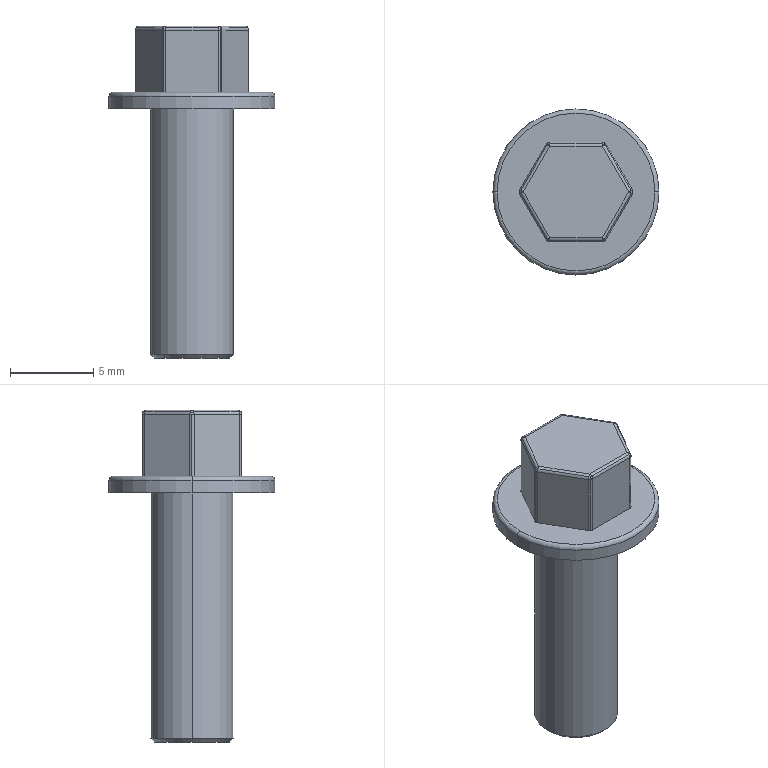Part | SolidWorks | features BaseBody 1 | 1 solid | 54 faces | box 10 x 10 x 20 mm | volume 496.617 mm3 | cylinder 28 | sphere 12 | plane 10 | cone 2 | torus 2 | commonest cylinder face diameters 0.5 x24 5 x2 10 x2
STEP:
#1=CARTESIAN_POINT('',(2.275,0.,-15.));
#2=VERTEX_POINT('',#1);
#3=CARTESIAN_POINT('',(-2.275,0.,-15.));
#4=VERTEX_POINT('',#3);
#5=CARTESIAN_POINT('',(0.,0.,-15.));
#6=DIRECTION('',(0.,0.,1.));
#7=DIRECTION('',(1.,0.,0.));
#8=AXIS2_PLACEMENT_3D('',#5,#6,#7);
#9=CIRCLE('',#8,2.275);
#10=EDGE_CURVE('',#2,#4,#9,.T.);
#11=ORIENTED_EDGE('',*,*,#10,.T.);
#12=CARTESIAN_POINT('',(-2.5,0.,-14.775));
#13=VERTEX_POINT('',#12);
#14=CARTESIAN_POINT('',(-2.387,0.,-14.887));
#15=DIRECTION('',(-0.7071,0.,0.7071));
#16=VECTOR('',#15,1000.);
#17=LINE('',#14,#16);
#18=EDGE_CURVE('',#4,#13,#17,.T.);
#19=ORIENTED_EDGE('',*,*,#18,.T.);
#20=CARTESIAN_POINT('',(2.5,0.,-14.775));
#21=VERTEX_POINT('',#20);
#22=CARTESIAN_POINT('',(0.,0.,-14.775));
#23=DIRECTION('',(0.,0.,-1.));
#24=DIRECTION('',(1.,0.,0.));
#25=AXIS2_PLACEMENT_3D('',#22,#23,#24);
#26=CIRCLE('',#25,2.5);
#27=EDGE_CURVE('',#13,#21,#26,.T.);
#28=ORIENTED_EDGE('',*,*,#27,.T.);
#29=CARTESIAN_POINT('',(2.387,0.,-14.887));
#30=DIRECTION('',(0.7071,0.,0.7071));
#31=VECTOR('',#30,1000.);
#32=LINE('',#29,#31);
#33=EDGE_CURVE('',#2,#21,#32,.T.);
#34=ORIENTED_EDGE('',*,*,#33,.F.);
#35=EDGE_LOOP('',(#11,#19,#28,#34));
#36=FACE_OUTER_BOUND('',#35,.T.);
#37=CARTESIAN_POINT('',(0.,0.,-14.887));
#38=DIRECTION('',(0.,0.,1.));
#39=DIRECTION('',(1.,0.,0.));
#40=AXIS2_PLACEMENT_3D('',#37,#38,#39);
#41=CONICAL_SURFACE('',#40,2.387,0.7854);
#42=ADVANCED_FACE('',(#36),#41,.T.);
#43=ORIENTED_EDGE('',*,*,#27,.F.);
#44=CARTESIAN_POINT('',(-2.5,0.,0.));
#45=VERTEX_POINT('',#44);
#46=CARTESIAN_POINT('',(-2.5,0.,0.));
#47=DIRECTION('',(0.,0.,1.));
#48=VECTOR('',#47,1000.);
#49=LINE('',#46,#48);
#50=EDGE_CURVE('',#13,#45,#49,.T.);
#51=ORIENTED_EDGE('',*,*,#50,.T.);
#52=CARTESIAN_POINT('',(2.5,0.,0.));
#53=VERTEX_POINT('',#52);
#54=CARTESIAN_POINT('',(0.,0.,0.));
#55=DIRECTION('',(0.,0.,1.));
#56=DIRECTION('',(1.,0.,0.));
#57=AXIS2_PLACEMENT_3D('',#54,#55,#56);
#58=CIRCLE('',#57,2.5);
#59=EDGE_CURVE('',#53,#45,#58,.T.);
#60=ORIENTED_EDGE('',*,*,#59,.F.);
#61=CARTESIAN_POINT('',(2.5,0.,0.));
#62=DIRECTION('',(0.,0.,1.));
#63=VECTOR('',#62,1000.);
#64=LINE('',#61,#63);
#65=EDGE_CURVE('',#21,#53,#64,.T.);
#66=ORIENTED_EDGE('',*,*,#65,.F.);
#67=EDGE_LOOP('',(#43,#51,#60,#66));
#68=FACE_OUTER_BOUND('',#67,.T.);
#69=CARTESIAN_POINT('',(0.,0.,0.));
#70=DIRECTION('',(0.,0.,1.));
#71=DIRECTION('',(1.,0.,0.));
#72=AXIS2_PLACEMENT_3D('',#69,#70,#71);
#73=CYLINDRICAL_SURFACE('',#72,2.5);
#74=ADVANCED_FACE('',(#68),#73,.T.);
#75=CARTESIAN_POINT('',(-1.681,-2.982,4.75));
#76=VERTEX_POINT('',#75);
#77=CARTESIAN_POINT('',(-1.713,-2.967,4.75));
#78=VERTEX_POINT('',#77);
#79=CARTESIAN_POINT('',(-1.588,-2.75,4.75));
#80=DIRECTION('',(0.,0.,-1.));
#81=DIRECTION('',(0.,-1.,0.));
#82=AXIS2_PLACEMENT_3D('',#79,#80,#81);
#83=CIRCLE('',#82,0.25);
#84=EDGE_CURVE('',#76,#78,#83,.T.);
#85=ORIENTED_EDGE('',*,*,#84,.F.);
#86=CARTESIAN_POINT('',(-1.668,-2.796,4.982));
#87=VERTEX_POINT('',#86);
#88=CARTESIAN_POINT('',(-1.588,-2.75,4.75));
#89=DIRECTION('',(-0.9014,0.3603,-0.2402));
#90=DIRECTION('',(-0.3712,-0.9286,0.));
#91=AXIS2_PLACEMENT_3D('',#88,#89,#90);
#92=CIRCLE('',#91,0.25);
#93=EDGE_CURVE('',#76,#87,#92,.T.);
#94=ORIENTED_EDGE('',*,*,#93,.T.);
#95=CARTESIAN_POINT('',(-1.741,-2.838,4.927));
#96=VERTEX_POINT('',#95);
#97=CARTESIAN_POINT('',(-1.588,-2.75,4.75));
#98=DIRECTION('',(-0.5,0.866,0.));
#99=DIRECTION('',(-0.866,-0.5,0.));
#100=AXIS2_PLACEMENT_3D('',#97,#98,#99);
#101=CIRCLE('',#100,0.25);
#102=EDGE_CURVE('',#96,#87,#101,.T.);
#103=ORIENTED_EDGE('',*,*,#102,.F.);
#104=CARTESIAN_POINT('',(-1.804,-2.875,4.75));
#105=VERTEX_POINT('',#104);
#106=CARTESIAN_POINT('',(-1.588,-2.75,4.75));
#107=DIRECTION('',(-0.5,0.866,0.));
#108=DIRECTION('',(-0.866,-0.5,0.));
#109=AXIS2_PLACEMENT_3D('',#106,#107,#108);
#110=CIRCLE('',#109,0.25);
#111=EDGE_CURVE('',#105,#96,#110,.T.);
#112=ORIENTED_EDGE('',*,*,#111,.F.);
#113=CARTESIAN_POINT('',(-1.588,-2.75,4.75));
#114=DIRECTION('',(0.,0.,-1.));
#115=DIRECTION('',(0.,-1.,0.));
#116=AXIS2_PLACEMENT_3D('',#113,#114,#115);
#117=CIRCLE('',#116,0.25);
#118=EDGE_CURVE('',#78,#105,#117,.T.);
#119=ORIENTED_EDGE('',*,*,#118,.F.);
#120=EDGE_LOOP('',(#85,#94,#103,#112,#119));
#121=FACE_OUTER_BOUND('',#120,.T.);
#122=CARTESIAN_POINT('',(-1.588,-2.75,4.75));
#123=DIRECTION('',(0.9014,-0.3603,0.2402));
#124=DIRECTION('',(-0.433,-0.75,0.5));
#125=AXIS2_PLACEMENT_3D('',#122,#123,#124);
#126=SPHERICAL_SURFACE('',#125,0.25);
#127=ADVANCED_FACE('',(#121),#126,.T.);
#128=CARTESIAN_POINT('',(1.681,-2.982,4.75));
#129=VERTEX_POINT('',#128);
#130=CARTESIAN_POINT('',(1.588,-3.,4.75));
#131=VERTEX_POINT('',#130);
#132=CARTESIAN_POINT('',(1.588,-2.75,4.75));
#133=DIRECTION('',(0.,0.,-1.));
#134=DIRECTION('',(0.866,-0.5,0.));
#135=AXIS2_PLACEMENT_3D('',#132,#133,#134);
#136=CIRCLE('',#135,0.25);
#137=EDGE_CURVE('',#129,#131,#136,.T.);
#138=ORIENTED_EDGE('',*,*,#137,.F.);
#139=CARTESIAN_POINT('',(1.668,-2.796,4.982));
#140=VERTEX_POINT('',#139);
#141=CARTESIAN_POINT('',(1.588,-2.75,4.75));
#142=DIRECTION('',(-0.9014,-0.3603,0.2402));
#143=DIRECTION('',(0.3712,-0.9286,0.));
#144=AXIS2_PLACEMENT_3D('',#141,#142,#143);
#145=CIRCLE('',#144,0.25);
#146=EDGE_CURVE('',#129,#140,#145,.T.);
#147=ORIENTED_EDGE('',*,*,#146,.T.);
#148=CARTESIAN_POINT('',(1.588,-2.75,5.));
#149=VERTEX_POINT('',#148);
#150=CARTESIAN_POINT('',(1.588,-2.75,4.75));
#151=DIRECTION('',(0.5,0.866,0.));
#152=DIRECTION('',(0.,0.,1.));
#153=AXIS2_PLACEMENT_3D('',#150,#151,#152);
#154=CIRCLE('',#153,0.25);
#155=EDGE_CURVE('',#149,#140,#154,.T.);
#156=ORIENTED_EDGE('',*,*,#155,.F.);
#157=CARTESIAN_POINT('',(1.588,-2.927,4.927));
#158=VERTEX_POINT('',#157);
#159=CARTESIAN_POINT('',(1.588,-2.75,4.75));
#160=DIRECTION('',(-1.,0.,0.));
#161=DIRECTION('',(0.,-1.,0.));
#162=AXIS2_PLACEMENT_3D('',#159,#160,#161);
#163=CIRCLE('',#162,0.25);
#164=EDGE_CURVE('',#158,#149,#163,.T.);
#165=ORIENTED_EDGE('',*,*,#164,.F.);
#166=CARTESIAN_POINT('',(1.588,-2.75,4.75));
#167=DIRECTION('',(-1.,0.,0.));
#168=DIRECTION('',(0.,-1.,0.));
#169=AXIS2_PLACEMENT_3D('',#166,#167,#168);
#170=CIRCLE('',#169,0.25);
#171=EDGE_CURVE('',#131,#158,#170,.T.);
#172=ORIENTED_EDGE('',*,*,#171,.F.);
#173=EDGE_LOOP('',(#138,#147,#156,#165,#172));
#174=FACE_OUTER_BOUND('',#173,.T.);
#175=CARTESIAN_POINT('',(1.588,-2.75,4.75));
#176=DIRECTION('',(0.9014,0.3603,-0.2402));
#177=DIRECTION('',(0.433,-0.75,0.5));
#178=AXIS2_PLACEMENT_3D('',#175,#176,#177);
#179=SPHERICAL_SURFACE('',#178,0.25);
#180=ADVANCED_FACE('',(#174),#179,.T.);
#181=CARTESIAN_POINT('',(-3.369,-0.1118,4.862));
#182=VERTEX_POINT('',#181);
#183=CARTESIAN_POINT('',(-3.392,-0.125,4.75));
#184=VERTEX_POINT('',#183);
#185=CARTESIAN_POINT('',(-3.175,0.,4.75));
#186=DIRECTION('',(0.5,-0.866,0.));
#187=DIRECTION('',(0.,0.,1.));
#188=AXIS2_PLACEMENT_3D('',#185,#186,#187);
#189=CIRCLE('',#188,0.25);
#190=EDGE_CURVE('',#182,#184,#189,.T.);
#191=ORIENTED_EDGE('',*,*,#190,.F.);
#192=CARTESIAN_POINT('',(-3.369,0.1118,4.862));
#193=VERTEX_POINT('',#192);
#194=CARTESIAN_POINT('',(-3.175,0.,4.75));
#195=DIRECTION('',(-0.5,0.,-0.866));
#196=DIRECTION('',(-0.866,0.,0.5));
#197=AXIS2_PLACEMENT_3D('',#194,#195,#196);
#198=CIRCLE('',#197,0.25);
#199=EDGE_CURVE('',#182,#193,#198,.T.);
#200=ORIENTED_EDGE('',*,*,#199,.T.);
#201=CARTESIAN_POINT('',(-3.392,0.125,4.75));
#202=VERTEX_POINT('',#201);
#203=CARTESIAN_POINT('',(-3.175,0.,4.75));
#204=DIRECTION('',(0.5,0.866,0.));
#205=DIRECTION('',(-0.866,0.5,0.));
#206=AXIS2_PLACEMENT_3D('',#203,#204,#205);
#207=CIRCLE('',#206,0.25);
#208=EDGE_CURVE('',#202,#193,#207,.T.);
#209=ORIENTED_EDGE('',*,*,#208,.F.);
#210=CARTESIAN_POINT('',(-3.425,0.,4.75));
#211=VERTEX_POINT('',#210);
#212=CARTESIAN_POINT('',(-3.175,0.,4.75));
#213=DIRECTION('',(0.,0.,-1.));
#214=DIRECTION('',(-0.866,-0.5,0.));
#215=AXIS2_PLACEMENT_3D('',#212,#213,#214);
#216=CIRCLE('',#215,0.25);
#217=EDGE_CURVE('',#211,#202,#216,.T.);
#218=ORIENTED_EDGE('',*,*,#217,.F.);
#219=CARTESIAN_POINT('',(-3.175,0.,4.75));
#220=DIRECTION('',(0.,0.,-1.));
#221=DIRECTION('',(-0.866,-0.5,0.));
#222=AXIS2_PLACEMENT_3D('',#219,#220,#221);
#223=CIRCLE('',#222,0.25);
#224=EDGE_CURVE('',#184,#211,#223,.T.);
#225=ORIENTED_EDGE('',*,*,#224,.F.);
#226=EDGE_LOOP('',(#191,#200,#209,#218,#225));
#227=FACE_OUTER_BOUND('',#226,.T.);
#228=CARTESIAN_POINT('',(-3.175,0.,4.75));
#229=DIRECTION('',(0.5,0.,0.866));
#230=DIRECTION('',(-0.866,0.,0.5));
#231=AXIS2_PLACEMENT_3D('',#228,#229,#230);
#232=SPHERICAL_SURFACE('',#231,0.25);
#233=ADVANCED_FACE('',(#227),#232,.T.);
#234=CARTESIAN_POINT('',(3.369,0.1118,4.862));
#235=VERTEX_POINT('',#234);
#236=CARTESIAN_POINT('',(3.392,0.125,4.75));
#237=VERTEX_POINT('',#236);
#238=CARTESIAN_POINT('',(3.175,0.,4.75));
#239=DIRECTION('',(-0.5,0.866,0.));
#240=DIRECTION('',(0.,0.,1.));
#241=AXIS2_PLACEMENT_3D('',#238,#239,#240);
#242=CIRCLE('',#241,0.25);
#243=EDGE_CURVE('',#235,#237,#242,.T.);
#244=ORIENTED_EDGE('',*,*,#243,.F.);
#245=CARTESIAN_POINT('',(3.369,-0.1118,4.862));
#246=VERTEX_POINT('',#245);
#247=CARTESIAN_POINT('',(3.175,0.,4.75));
#248=DIRECTION('',(0.5,0.,-0.866));
#249=DIRECTION('',(-0.866,0.,-0.5));
#250=AXIS2_PLACEMENT_3D('',#247,#248,#249);
#251=CIRCLE('',#250,0.25);
#252=EDGE_CURVE('',#235,#246,#251,.T.);
#253=ORIENTED_EDGE('',*,*,#252,.T.);
#254=CARTESIAN_POINT('',(3.392,-0.125,4.75));
#255=VERTEX_POINT('',#254);
#256=CARTESIAN_POINT('',(3.175,0.,4.75));
#257=DIRECTION('',(-0.5,-0.866,0.));
#258=DIRECTION('',(0.866,-0.5,0.));
#259=AXIS2_PLACEMENT_3D('',#256,#257,#258);
#260=CIRCLE('',#259,0.25);
#261=EDGE_CURVE('',#255,#246,#260,.T.);
#262=ORIENTED_EDGE('',*,*,#261,.F.);
#263=CARTESIAN_POINT('',(3.425,0.,4.75));
#264=VERTEX_POINT('',#263);
#265=CARTESIAN_POINT('',(3.175,0.,4.75));
#266=DIRECTION('',(0.,0.,-1.));
#267=DIRECTION('',(0.866,0.5,0.));
#268=AXIS2_PLACEMENT_3D('',#265,#266,#267);
#269=CIRCLE('',#268,0.25);
#270=EDGE_CURVE('',#264,#255,#269,.T.);
#271=ORIENTED_EDGE('',*,*,#270,.F.);
#272=CARTESIAN_POINT('',(3.175,0.,4.75));
#273=DIRECTION('',(0.,0.,-1.));
#274=DIRECTION('',(0.866,0.5,0.));
#275=AXIS2_PLACEMENT_3D('',#272,#273,#274);
#276=CIRCLE('',#275,0.25);
#277=EDGE_CURVE('',#237,#264,#276,.T.);
#278=ORIENTED_EDGE('',*,*,#277,.F.);
#279=EDGE_LOOP('',(#244,#253,#262,#271,#278));
#280=FACE_OUTER_BOUND('',#279,.T.);
#281=CARTESIAN_POINT('',(3.175,0.,4.75));
#282=DIRECTION('',(-0.5,0.,0.866));
#283=DIRECTION('',(0.866,0.,0.5));
#284=AXIS2_PLACEMENT_3D('',#281,#282,#283);
#285=SPHERICAL_SURFACE('',#284,0.25);
#286=ADVANCED_FACE('',(#280),#285,.T.);
#287=ORIENTED_EDGE('',*,*,#261,.T.);
#288=CARTESIAN_POINT('',(3.329,-0.08839,4.927));
#289=VERTEX_POINT('',#288);
#290=CARTESIAN_POINT('',(3.175,0.,4.75));
#291=DIRECTION('',(-0.5,-0.866,0.));
#292=DIRECTION('',(0.866,-0.5,0.));
#293=AXIS2_PLACEMENT_3D('',#290,#291,#292);
#294=CIRCLE('',#293,0.25);
#295=EDGE_CURVE('',#246,#289,#294,.T.);
#296=ORIENTED_EDGE('',*,*,#295,.T.);
#297=CARTESIAN_POINT('',(1.741,-2.838,4.927));
#298=VERTEX_POINT('',#297);
#299=CARTESIAN_POINT('',(2.968,-0.7134,4.927));
#300=DIRECTION('',(-0.5,-0.866,0.));
#301=VECTOR('',#300,1000.);
#302=LINE('',#299,#301);
#303=EDGE_CURVE('',#289,#298,#302,.T.);
#304=ORIENTED_EDGE('',*,*,#303,.T.);
#305=CARTESIAN_POINT('',(1.804,-2.875,4.75));
#306=VERTEX_POINT('',#305);
#307=CARTESIAN_POINT('',(1.588,-2.75,4.75));
#308=DIRECTION('',(0.5,0.866,0.));
#309=DIRECTION('',(0.,0.,1.));
#310=AXIS2_PLACEMENT_3D('',#307,#308,#309);
#311=CIRCLE('',#310,0.25);
#312=EDGE_CURVE('',#298,#306,#311,.T.);
#313=ORIENTED_EDGE('',*,*,#312,.T.);
#314=CARTESIAN_POINT('',(3.031,-0.75,4.75));
#315=DIRECTION('',(0.5,0.866,0.));
#316=VECTOR('',#315,1000.);
#317=LINE('',#314,#316);
#318=EDGE_CURVE('',#306,#255,#317,.T.);
#319=ORIENTED_EDGE('',*,*,#318,.T.);
#320=EDGE_LOOP('',(#287,#296,#304,#313,#319));
#321=FACE_OUTER_BOUND('',#320,.T.);
#322=CARTESIAN_POINT('',(2.815,-0.625,4.75));
#323=DIRECTION('',(-0.5,-0.866,0.));
#324=DIRECTION('',(0.6124,-0.3536,0.7071));
#325=AXIS2_PLACEMENT_3D('',#322,#323,#324);
#326=CYLINDRICAL_SURFACE('',#325,0.25);
#327=ADVANCED_FACE('',(#321),#326,.T.);
#328=CARTESIAN_POINT('',(3.392,-0.125,1.));
#329=VERTEX_POINT('',#328);
#330=CARTESIAN_POINT('',(3.425,0.,1.));
#331=VERTEX_POINT('',#330);
#332=CARTESIAN_POINT('',(3.175,0.,1.));
#333=DIRECTION('',(0.,0.,1.));
#334=DIRECTION('',(1.,0.,0.));
#335=AXIS2_PLACEMENT_3D('',#332,#333,#334);
#336=CIRCLE('',#335,0.25);
#337=EDGE_CURVE('',#329,#331,#336,.T.);
#338=ORIENTED_EDGE('',*,*,#337,.T.);
#339=CARTESIAN_POINT('',(3.425,0.,5.));
#340=DIRECTION('',(0.,0.,1.));
#341=VECTOR('',#340,1000.);
#342=LINE('',#339,#341);
#343=EDGE_CURVE('',#331,#264,#342,.T.);
#344=ORIENTED_EDGE('',*,*,#343,.T.);
#345=ORIENTED_EDGE('',*,*,#270,.T.);
#346=CARTESIAN_POINT('',(3.392,-0.125,5.));
#347=DIRECTION('',(0.,0.,-1.));
#348=VECTOR('',#347,1000.);
#349=LINE('',#346,#348);
#350=EDGE_CURVE('',#255,#329,#349,.T.);
#351=ORIENTED_EDGE('',*,*,#350,.T.);
#352=EDGE_LOOP('',(#338,#344,#345,#351));
#353=FACE_OUTER_BOUND('',#352,.T.);
#354=CARTESIAN_POINT('',(3.175,0.,5.));
#355=DIRECTION('',(0.,0.,1.));
#356=DIRECTION('',(1.,0.,0.));
#357=AXIS2_PLACEMENT_3D('',#354,#355,#356);
#358=CYLINDRICAL_SURFACE('',#357,0.25);
#359=ADVANCED_FACE('',(#353),#358,.T.);
#360=CARTESIAN_POINT('',(-1.668,2.796,4.982));
#361=VERTEX_POINT('',#360);
#362=CARTESIAN_POINT('',(-1.741,2.838,4.927));
#363=VERTEX_POINT('',#362);
#364=CARTESIAN_POINT('',(-1.588,2.75,4.75));
#365=DIRECTION('',(-0.5,-0.866,0.));
#366=DIRECTION('',(0.,0.,1.));
#367=AXIS2_PLACEMENT_3D('',#364,#365,#366);
#368=CIRCLE('',#367,0.25);
#369=EDGE_CURVE('',#361,#363,#368,.T.);
#370=ORIENTED_EDGE('',*,*,#369,.F.);
#371=CARTESIAN_POINT('',(-1.681,2.982,4.75));
#372=VERTEX_POINT('',#371);
#373=CARTESIAN_POINT('',(-1.588,2.75,4.75));
#374=DIRECTION('',(-0.9014,-0.3603,-0.2402));
#375=DIRECTION('',(0.3712,-0.9286,0.));
#376=AXIS2_PLACEMENT_3D('',#373,#374,#375);
#377=CIRCLE('',#376,0.25);
#378=EDGE_CURVE('',#361,#372,#377,.T.);
#379=ORIENTED_EDGE('',*,*,#378,.T.);
#380=CARTESIAN_POINT('',(-1.713,2.967,4.75));
#381=VERTEX_POINT('',#380);
#382=CARTESIAN_POINT('',(-1.588,2.75,4.75));
#383=DIRECTION('',(0.,0.,-1.));
#384=DIRECTION('',(-0.866,0.5,0.));
#385=AXIS2_PLACEMENT_3D('',#382,#383,#384);
#386=CIRCLE('',#385,0.25);
#387=EDGE_CURVE('',#381,#372,#386,.T.);
#388=ORIENTED_EDGE('',*,*,#387,.F.);
#389=CARTESIAN_POINT('',(-1.804,2.875,4.75));
#390=VERTEX_POINT('',#389);
#391=CARTESIAN_POINT('',(-1.588,2.75,4.75));
#392=DIRECTION('',(0.,0.,-1.));
#393=DIRECTION('',(-0.866,0.5,0.));
#394=AXIS2_PLACEMENT_3D('',#391,#392,#393);
#395=CIRCLE('',#394,0.25);
#396=EDGE_CURVE('',#390,#381,#395,.T.);
#397=ORIENTED_EDGE('',*,*,#396,.F.);
#398=CARTESIAN_POINT('',(-1.588,2.75,4.75));
#399=DIRECTION('',(-0.5,-0.866,0.));
#400=DIRECTION('',(0.,0.,1.));
#401=AXIS2_PLACEMENT_3D('',#398,#399,#400);
#402=CIRCLE('',#401,0.25);
#403=EDGE_CURVE('',#363,#390,#402,.T.);
#404=ORIENTED_EDGE('',*,*,#403,.F.);
#405=EDGE_LOOP('',(#370,#379,#388,#397,#404));
#406=FACE_OUTER_BOUND('',#405,.T.);
#407=CARTESIAN_POINT('',(-1.588,2.75,4.75));
#408=DIRECTION('',(0.9014,0.3603,0.2402));
#409=DIRECTION('',(-0.433,0.75,0.5));
#410=AXIS2_PLACEMENT_3D('',#407,#408,#409);
#411=SPHERICAL_SURFACE('',#410,0.25);
#412=ADVANCED_FACE('',(#406),#411,.T.);
#413=CARTESIAN_POINT('',(1.668,2.796,4.982));
#414=VERTEX_POINT('',#413);
#415=CARTESIAN_POINT('',(1.588,2.75,5.));
#416=VERTEX_POINT('',#415);
#417=CARTESIAN_POINT('',(1.588,2.75,4.75));
#418=DIRECTION('',(0.5,-0.866,0.));
#419=DIRECTION('',(0.866,0.5,0.));
#420=AXIS2_PLACEMENT_3D('',#417,#418,#419);
#421=CIRCLE('',#420,0.25);
#422=EDGE_CURVE('',#414,#416,#421,.T.);
#423=ORIENTED_EDGE('',*,*,#422,.F.);
#424=CARTESIAN_POINT('',(1.681,2.982,4.75));
#425=VERTEX_POINT('',#424);
#426=CARTESIAN_POINT('',(1.588,2.75,4.75));
#427=DIRECTION('',(-0.9014,0.3603,0.2402));
#428=DIRECTION('',(-0.3712,-0.9286,0.));
#429=AXIS2_PLACEMENT_3D('',#426,#427,#428);
#430=CIRCLE('',#429,0.25);
#431=EDGE_CURVE('',#414,#425,#430,.T.);
#432=ORIENTED_EDGE('',*,*,#431,.T.);
#433=CARTESIAN_POINT('',(1.588,3.,4.75));
#434=VERTEX_POINT('',#433);
#435=CARTESIAN_POINT('',(1.588,2.75,4.75));
#436=DIRECTION('',(0.,0.,-1.));
#437=DIRECTION('',(0.,1.,0.));
#438=AXIS2_PLACEMENT_3D('',#435,#436,#437);
#439=CIRCLE('',#438,0.25);
#440=EDGE_CURVE('',#434,#425,#439,.T.);
#441=ORIENTED_EDGE('',*,*,#440,.F.);
#442=CARTESIAN_POINT('',(1.588,2.927,4.927));
#443=VERTEX_POINT('',#442);
#444=CARTESIAN_POINT('',(1.588,2.75,4.75));
#445=DIRECTION('',(-1.,0.,0.));
#446=DIRECTION('',(0.,0.,1.));
#447=AXIS2_PLACEMENT_3D('',#444,#445,#446);
#448=CIRCLE('',#447,0.25);
#449=EDGE_CURVE('',#443,#434,#448,.T.);
#450=ORIENTED_EDGE('',*,*,#449,.F.);
#451=CARTESIAN_POINT('',(1.588,2.75,4.75));
#452=DIRECTION('',(-1.,0.,0.));
#453=DIRECTION('',(0.,0.,1.));
#454=AXIS2_PLACEMENT_3D('',#451,#452,#453);
#455=CIRCLE('',#454,0.25);
#456=EDGE_CURVE('',#416,#443,#455,.T.);
#457=ORIENTED_EDGE('',*,*,#456,.F.);
#458=EDGE_LOOP('',(#423,#432,#441,#450,#457));
#459=FACE_OUTER_BOUND('',#458,.T.);
#460=CARTESIAN_POINT('',(1.588,2.75,4.75));
#461=DIRECTION('',(0.9014,-0.3603,-0.2402));
#462=DIRECTION('',(0.433,0.75,0.5));
#463=AXIS2_PLACEMENT_3D('',#460,#461,#462);
#464=SPHERICAL_SURFACE('',#463,0.25);
#465=ADVANCED_FACE('',(#459),#464,.T.);
#466=CARTESIAN_POINT('',(1.804,2.875,4.75));
#467=VERTEX_POINT('',#466);
#468=CARTESIAN_POINT('',(1.741,2.838,4.927));
#469=VERTEX_POINT('',#468);
#470=CARTESIAN_POINT('',(1.588,2.75,4.75));
#471=DIRECTION('',(0.5,-0.866,0.));
#472=DIRECTION('',(0.866,0.5,0.));
#473=AXIS2_PLACEMENT_3D('',#470,#471,#472);
#474=CIRCLE('',#473,0.25);
#475=EDGE_CURVE('',#467,#469,#474,.T.);
#476=ORIENTED_EDGE('',*,*,#475,.T.);
#477=CARTESIAN_POINT('',(3.329,0.08839,4.927));
#478=VERTEX_POINT('',#477);
#479=CARTESIAN_POINT('',(2.102,2.213,4.927));
#480=DIRECTION('',(0.5,-0.866,0.));
#481=VECTOR('',#480,1000.);
#482=LINE('',#479,#481);
#483=EDGE_CURVE('',#469,#478,#482,.T.);
#484=ORIENTED_EDGE('',*,*,#483,.T.);
#485=CARTESIAN_POINT('',(3.175,0.,4.75));
#486=DIRECTION('',(-0.5,0.866,0.));
#487=DIRECTION('',(0.,0.,1.));
#488=AXIS2_PLACEMENT_3D('',#485,#486,#487);
#489=CIRCLE('',#488,0.25);
#490=EDGE_CURVE('',#478,#235,#489,.T.);
#491=ORIENTED_EDGE('',*,*,#490,.T.);
#492=ORIENTED_EDGE('',*,*,#243,.T.);
#493=CARTESIAN_POINT('',(2.165,2.25,4.75));
#494=DIRECTION('',(-0.5,0.866,0.));
#495=VECTOR('',#494,1000.);
#496=LINE('',#493,#495);
#497=EDGE_CURVE('',#237,#467,#496,.T.);
#498=ORIENTED_EDGE('',*,*,#497,.T.);
#499=EDGE_LOOP('',(#476,#484,#491,#492,#498));
#500=FACE_OUTER_BOUND('',#499,.T.);
#501=CARTESIAN_POINT('',(1.949,2.125,4.75));
#502=DIRECTION('',(0.5,-0.866,0.));
#503=DIRECTION('',(0.6124,0.3536,0.7071));
#504=AXIS2_PLACEMENT_3D('',#501,#502,#503);
#505=CYLINDRICAL_SURFACE('',#504,0.25);
#506=ADVANCED_FACE('',(#500),#505,.T.);
#507=CARTESIAN_POINT('',(1.804,2.875,1.));
#508=VERTEX_POINT('',#507);
#509=CARTESIAN_POINT('',(1.713,2.967,1.));
#510=VERTEX_POINT('',#509);
#511=CARTESIAN_POINT('',(1.588,2.75,1.));
#512=DIRECTION('',(0.,0.,1.));
#513=DIRECTION('',(0.5,0.866,0.));
#514=AXIS2_PLACEMENT_3D('',#511,#512,#513);
#515=CIRCLE('',#514,0.25);
#516=EDGE_CURVE('',#508,#510,#515,.T.);
#517=ORIENTED_EDGE('',*,*,#516,.T.);
#518=CARTESIAN_POINT('',(1.713,2.967,4.75));
#519=VERTEX_POINT('',#518);
#520=CARTESIAN_POINT('',(1.713,2.967,5.));
#521=DIRECTION('',(0.,0.,1.));
#522=VECTOR('',#521,1000.);
#523=LINE('',#520,#522);
#524=EDGE_CURVE('',#510,#519,#523,.T.);
#525=ORIENTED_EDGE('',*,*,#524,.T.);
#526=CARTESIAN_POINT('',(1.588,2.75,4.75));
#527=DIRECTION('',(0.,0.,-1.));
#528=DIRECTION('',(0.,1.,0.));
#529=AXIS2_PLACEMENT_3D('',#526,#527,#528);
#530=CIRCLE('',#529,0.25);
#531=EDGE_CURVE('',#519,#467,#530,.T.);
#532=ORIENTED_EDGE('',*,*,#531,.T.);
#533=CARTESIAN_POINT('',(1.804,2.875,5.));
#534=DIRECTION('',(0.,0.,-1.));
#535=VECTOR('',#534,1000.);
#536=LINE('',#533,#535);
#537=EDGE_CURVE('',#467,#508,#536,.T.);
#538=ORIENTED_EDGE('',*,*,#537,.T.);
#539=EDGE_LOOP('',(#517,#525,#532,#538));
#540=FACE_OUTER_BOUND('',#539,.T.);
#541=CARTESIAN_POINT('',(1.588,2.75,5.));
#542=DIRECTION('',(0.,0.,1.));
#543=DIRECTION('',(0.5,0.866,0.));
#544=AXIS2_PLACEMENT_3D('',#541,#542,#543);
#545=CYLINDRICAL_SURFACE('',#544,0.25);
#546=ADVANCED_FACE('',(#540),#545,.T.);
#547=CARTESIAN_POINT('',(-1.588,3.,4.75));
#548=VERTEX_POINT('',#547);
#549=CARTESIAN_POINT('',(-1.588,2.927,4.927));
#550=VERTEX_POINT('',#549);
#551=CARTESIAN_POINT('',(-1.588,2.75,4.75));
#552=DIRECTION('',(1.,0.,0.));
#553=DIRECTION('',(0.,1.,0.));
#554=AXIS2_PLACEMENT_3D('',#551,#552,#553);
#555=CIRCLE('',#554,0.25);
#556=EDGE_CURVE('',#548,#550,#555,.T.);
#557=ORIENTED_EDGE('',*,*,#556,.T.);
#558=CARTESIAN_POINT('',(-0.866,2.927,4.927));
#559=DIRECTION('',(1.,0.,0.));
#560=VECTOR('',#559,1000.);
#561=LINE('',#558,#560);
#562=EDGE_CURVE('',#550,#443,#561,.T.);
#563=ORIENTED_EDGE('',*,*,#562,.T.);
#564=ORIENTED_EDGE('',*,*,#449,.T.);
#565=CARTESIAN_POINT('',(-0.866,3.,4.75));
#566=DIRECTION('',(-1.,0.,0.));
#567=VECTOR('',#566,1000.);
#568=LINE('',#565,#567);
#569=EDGE_CURVE('',#434,#548,#568,.T.);
#570=ORIENTED_EDGE('',*,*,#569,.T.);
#571=EDGE_LOOP('',(#557,#563,#564,#570));
#572=FACE_OUTER_BOUND('',#571,.T.);
#573=CARTESIAN_POINT('',(-0.866,2.75,4.75));
#574=DIRECTION('',(1.,0.,0.));
#575=DIRECTION('',(0.,0.7071,0.7071));
#576=AXIS2_PLACEMENT_3D('',#573,#574,#575);
#577=CYLINDRICAL_SURFACE('',#576,0.25);
#578=ADVANCED_FACE('',(#572),#577,.T.);
#579=CARTESIAN_POINT('',(-1.588,3.,1.));
#580=VERTEX_POINT('',#579);
#581=CARTESIAN_POINT('',(-1.713,2.967,1.));
#582=VERTEX_POINT('',#581);
#583=CARTESIAN_POINT('',(-1.588,2.75,1.));
#584=DIRECTION('',(0.,0.,1.));
#585=DIRECTION('',(-0.5,0.866,0.));
#586=AXIS2_PLACEMENT_3D('',#583,#584,#585);
#587=CIRCLE('',#586,0.25);
#588=EDGE_CURVE('',#580,#582,#587,.T.);
#589=ORIENTED_EDGE('',*,*,#588,.T.);
#590=CARTESIAN_POINT('',(-1.713,2.967,5.));
#591=DIRECTION('',(0.,0.,1.));
#592=VECTOR('',#591,1000.);
#593=LINE('',#590,#592);
#594=EDGE_CURVE('',#582,#381,#593,.T.);
#595=ORIENTED_EDGE('',*,*,#594,.T.);
#596=ORIENTED_EDGE('',*,*,#387,.T.);
#597=CARTESIAN_POINT('',(-1.588,2.75,4.75));
#598=DIRECTION('',(0.,0.,-1.));
#599=DIRECTION('',(-0.866,0.5,0.));
#600=AXIS2_PLACEMENT_3D('',#597,#598,#599);
#601=CIRCLE('',#600,0.25);
#602=EDGE_CURVE('',#372,#548,#601,.T.);
#603=ORIENTED_EDGE('',*,*,#602,.T.);
#604=CARTESIAN_POINT('',(-1.588,3.,5.));
#605=DIRECTION('',(0.,0.,-1.));
#606=VECTOR('',#605,1000.);
#607=LINE('',#604,#606);
#608=EDGE_CURVE('',#548,#580,#607,.T.);
#609=ORIENTED_EDGE('',*,*,#608,.T.);
#610=EDGE_LOOP('',(#589,#595,#596,#603,#609));
#611=FACE_OUTER_BOUND('',#610,.T.);
#612=CARTESIAN_POINT('',(-1.588,2.75,5.));
#613=DIRECTION('',(0.,0.,1.));
#614=DIRECTION('',(-0.5,0.866,0.));
#615=AXIS2_PLACEMENT_3D('',#612,#613,#614);
#616=CYLINDRICAL_SURFACE('',#615,0.25);
#617=ADVANCED_FACE('',(#611),#616,.T.);
#618=ORIENTED_EDGE('',*,*,#208,.T.);
#619=CARTESIAN_POINT('',(-3.329,0.08839,4.927));
#620=VERTEX_POINT('',#619);
#621=CARTESIAN_POINT('',(-3.175,0.,4.75));
#622=DIRECTION('',(0.5,0.866,0.));
#623=DIRECTION('',(-0.866,0.5,0.));
#624=AXIS2_PLACEMENT_3D('',#621,#622,#623);
#625=CIRCLE('',#624,0.25);
#626=EDGE_CURVE('',#193,#620,#625,.T.);
#627=ORIENTED_EDGE('',*,*,#626,.T.);
#628=CARTESIAN_POINT('',(-2.968,0.7134,4.927));
#629=DIRECTION('',(0.5,0.866,0.));
#630=VECTOR('',#629,1000.);
#631=LINE('',#628,#630);
#632=EDGE_CURVE('',#620,#363,#631,.T.);
#633=ORIENTED_EDGE('',*,*,#632,.T.);
#634=ORIENTED_EDGE('',*,*,#403,.T.);
#635=CARTESIAN_POINT('',(-3.031,0.75,4.75));
#636=DIRECTION('',(-0.5,-0.866,0.));
#637=VECTOR('',#636,1000.);
#638=LINE('',#635,#637);
#639=EDGE_CURVE('',#390,#202,#638,.T.);
#640=ORIENTED_EDGE('',*,*,#639,.T.);
#641=EDGE_LOOP('',(#618,#627,#633,#634,#640));
#642=FACE_OUTER_BOUND('',#641,.T.);
#643=CARTESIAN_POINT('',(-2.815,0.625,4.75));
#644=DIRECTION('',(0.5,0.866,0.));
#645=DIRECTION('',(-0.6124,0.3536,0.7071));
#646=AXIS2_PLACEMENT_3D('',#643,#644,#645);
#647=CYLINDRICAL_SURFACE('',#646,0.25);
#648=ADVANCED_FACE('',(#642),#647,.T.);
#649=CARTESIAN_POINT('',(-3.392,0.125,1.));
#650=VERTEX_POINT('',#649);
#651=CARTESIAN_POINT('',(-3.425,0.,1.));
#652=VERTEX_POINT('',#651);
#653=CARTESIAN_POINT('',(-3.175,0.,1.));
#654=DIRECTION('',(0.,0.,1.));
#655=DIRECTION('',(-1.,0.,0.));
#656=AXIS2_PLACEMENT_3D('',#653,#654,#655);
#657=CIRCLE('',#656,0.25);
#658=EDGE_CURVE('',#650,#652,#657,.T.);
#659=ORIENTED_EDGE('',*,*,#658,.T.);
#660=CARTESIAN_POINT('',(-3.425,0.,5.));
#661=DIRECTION('',(0.,0.,1.));
#662=VECTOR('',#661,1000.);
#663=LINE('',#660,#662);
#664=EDGE_CURVE('',#652,#211,#663,.T.);
#665=ORIENTED_EDGE('',*,*,#664,.T.);
#666=ORIENTED_EDGE('',*,*,#217,.T.);
#667=CARTESIAN_POINT('',(-3.392,0.125,5.));
#668=DIRECTION('',(0.,0.,-1.));
#669=VECTOR('',#668,1000.);
#670=LINE('',#667,#669);
#671=EDGE_CURVE('',#202,#650,#670,.T.);
#672=ORIENTED_EDGE('',*,*,#671,.T.);
#673=EDGE_LOOP('',(#659,#665,#666,#672));
#674=FACE_OUTER_BOUND('',#673,.T.);
#675=CARTESIAN_POINT('',(-3.175,0.,5.));
#676=DIRECTION('',(0.,0.,1.));
#677=DIRECTION('',(-1.,0.,0.));
#678=AXIS2_PLACEMENT_3D('',#675,#676,#677);
#679=CYLINDRICAL_SURFACE('',#678,0.25);
#680=ADVANCED_FACE('',(#674),#679,.T.);
#681=ORIENTED_EDGE('',*,*,#111,.T.);
#682=CARTESIAN_POINT('',(-3.329,-0.08839,4.927));
#683=VERTEX_POINT('',#682);
#684=CARTESIAN_POINT('',(-2.102,-2.213,4.927));
#685=DIRECTION('',(-0.5,0.866,0.));
#686=VECTOR('',#685,1000.);
#687=LINE('',#684,#686);
#688=EDGE_CURVE('',#96,#683,#687,.T.);
#689=ORIENTED_EDGE('',*,*,#688,.T.);
#690=CARTESIAN_POINT('',(-3.175,0.,4.75));
#691=DIRECTION('',(0.5,-0.866,0.));
#692=DIRECTION('',(0.,0.,1.));
#693=AXIS2_PLACEMENT_3D('',#690,#691,#692);
#694=CIRCLE('',#693,0.25);
#695=EDGE_CURVE('',#683,#182,#694,.T.);
#696=ORIENTED_EDGE('',*,*,#695,.T.);
#697=ORIENTED_EDGE('',*,*,#190,.T.);
#698=CARTESIAN_POINT('',(-2.165,-2.25,4.75));
#699=DIRECTION('',(0.5,-0.866,0.));
#700=VECTOR('',#699,1000.);
#701=LINE('',#698,#700);
#702=EDGE_CURVE('',#184,#105,#701,.T.);
#703=ORIENTED_EDGE('',*,*,#702,.T.);
#704=EDGE_LOOP('',(#681,#689,#696,#697,#703));
#705=FACE_OUTER_BOUND('',#704,.T.);
#706=CARTESIAN_POINT('',(-1.949,-2.125,4.75));
#707=DIRECTION('',(-0.5,0.866,0.));
#708=DIRECTION('',(-0.6124,-0.3536,0.7071));
#709=AXIS2_PLACEMENT_3D('',#706,#707,#708);
#710=CYLINDRICAL_SURFACE('',#709,0.25);
#711=ADVANCED_FACE('',(#705),#710,.T.);
#712=ORIENTED_EDGE('',*,*,#171,.T.);
#713=CARTESIAN_POINT('',(-1.588,-2.927,4.927));
#714=VERTEX_POINT('',#713);
#715=CARTESIAN_POINT('',(0.866,-2.927,4.927));
#716=DIRECTION('',(-1.,0.,0.));
#717=VECTOR('',#716,1000.);
#718=LINE('',#715,#717);
#719=EDGE_CURVE('',#158,#714,#718,.T.);
#720=ORIENTED_EDGE('',*,*,#719,.T.);
#721=CARTESIAN_POINT('',(-1.588,-3.,4.75));
#722=VERTEX_POINT('',#721);
#723=CARTESIAN_POINT('',(-1.588,-2.75,4.75));
#724=DIRECTION('',(1.,0.,0.));
#725=DIRECTION('',(0.,0.,1.));
#726=AXIS2_PLACEMENT_3D('',#723,#724,#725);
#727=CIRCLE('',#726,0.25);
#728=EDGE_CURVE('',#714,#722,#727,.T.);
#729=ORIENTED_EDGE('',*,*,#728,.T.);
#730=CARTESIAN_POINT('',(0.866,-3.,4.75));
#731=DIRECTION('',(1.,0.,0.));
#732=VECTOR('',#731,1000.);
#733=LINE('',#730,#732);
#734=EDGE_CURVE('',#722,#131,#733,.T.);
#735=ORIENTED_EDGE('',*,*,#734,.T.);
#736=EDGE_LOOP('',(#712,#720,#729,#735));
#737=FACE_OUTER_BOUND('',#736,.T.);
#738=CARTESIAN_POINT('',(0.866,-2.75,4.75));
#739=DIRECTION('',(-1.,0.,0.));
#740=DIRECTION('',(0.,-0.7071,0.7071));
#741=AXIS2_PLACEMENT_3D('',#738,#739,#740);
#742=CYLINDRICAL_SURFACE('',#741,0.25);
#743=ADVANCED_FACE('',(#737),#742,.T.);
#744=CARTESIAN_POINT('',(1.588,-3.,1.));
#745=VERTEX_POINT('',#744);
#746=CARTESIAN_POINT('',(1.713,-2.967,1.));
#747=VERTEX_POINT('',#746);
#748=CARTESIAN_POINT('',(1.588,-2.75,1.));
#749=DIRECTION('',(0.,0.,1.));
#750=DIRECTION('',(0.5,-0.866,0.));
#751=AXIS2_PLACEMENT_3D('',#748,#749,#750);
#752=CIRCLE('',#751,0.25);
#753=EDGE_CURVE('',#745,#747,#752,.T.);
#754=ORIENTED_EDGE('',*,*,#753,.T.);
#755=CARTESIAN_POINT('',(1.713,-2.967,4.75));
#756=VERTEX_POINT('',#755);
#757=CARTESIAN_POINT('',(1.713,-2.967,5.));
#758=DIRECTION('',(0.,0.,1.));
#759=VECTOR('',#758,1000.);
#760=LINE('',#757,#759);
#761=EDGE_CURVE('',#747,#756,#760,.T.);
#762=ORIENTED_EDGE('',*,*,#761,.T.);
#763=CARTESIAN_POINT('',(1.588,-2.75,4.75));
#764=DIRECTION('',(0.,0.,-1.));
#765=DIRECTION('',(0.866,-0.5,0.));
#766=AXIS2_PLACEMENT_3D('',#763,#764,#765);
#767=CIRCLE('',#766,0.25);
#768=EDGE_CURVE('',#756,#129,#767,.T.);
#769=ORIENTED_EDGE('',*,*,#768,.T.);
#770=ORIENTED_EDGE('',*,*,#137,.T.);
#771=CARTESIAN_POINT('',(1.588,-3.,5.));
#772=DIRECTION('',(0.,0.,-1.));
#773=VECTOR('',#772,1000.);
#774=LINE('',#771,#773);
#775=EDGE_CURVE('',#131,#745,#774,.T.);
#776=ORIENTED_EDGE('',*,*,#775,.T.);
#777=EDGE_LOOP('',(#754,#762,#769,#770,#776));
#778=FACE_OUTER_BOUND('',#777,.T.);
#779=CARTESIAN_POINT('',(1.588,-2.75,5.));
#780=DIRECTION('',(0.,0.,1.));
#781=DIRECTION('',(0.5,-0.866,0.));
#782=AXIS2_PLACEMENT_3D('',#779,#780,#781);
#783=CYLINDRICAL_SURFACE('',#782,0.25);
#784=ADVANCED_FACE('',(#778),#783,.T.);
#785=CARTESIAN_POINT('',(-1.804,-2.875,1.));
#786=VERTEX_POINT('',#785);
#787=CARTESIAN_POINT('',(-1.713,-2.967,1.));
#788=VERTEX_POINT('',#787);
#789=CARTESIAN_POINT('',(-1.588,-2.75,1.));
#790=DIRECTION('',(0.,0.,1.));
#791=DIRECTION('',(-0.5,-0.866,0.));
#792=AXIS2_PLACEMENT_3D('',#789,#790,#791);
#793=CIRCLE('',#792,0.25);
#794=EDGE_CURVE('',#786,#788,#793,.T.);
#795=ORIENTED_EDGE('',*,*,#794,.T.);
#796=CARTESIAN_POINT('',(-1.713,-2.967,5.));
#797=DIRECTION('',(0.,0.,1.));
#798=VECTOR('',#797,1000.);
#799=LINE('',#796,#798);
#800=EDGE_CURVE('',#788,#78,#799,.T.);
#801=ORIENTED_EDGE('',*,*,#800,.T.);
#802=ORIENTED_EDGE('',*,*,#118,.T.);
#803=CARTESIAN_POINT('',(-1.804,-2.875,5.));
#804=DIRECTION('',(0.,0.,-1.));
#805=VECTOR('',#804,1000.);
#806=LINE('',#803,#805);
#807=EDGE_CURVE('',#105,#786,#806,.T.);
#808=ORIENTED_EDGE('',*,*,#807,.T.);
#809=EDGE_LOOP('',(#795,#801,#802,#808));
#810=FACE_OUTER_BOUND('',#809,.T.);
#811=CARTESIAN_POINT('',(-1.588,-2.75,5.));
#812=DIRECTION('',(0.,0.,1.));
#813=DIRECTION('',(-0.5,-0.866,0.));
#814=AXIS2_PLACEMENT_3D('',#811,#812,#813);
#815=CYLINDRICAL_SURFACE('',#814,0.25);
#816=ADVANCED_FACE('',(#810),#815,.T.);
#817=CARTESIAN_POINT('',(-4.75,0.,1.));
#818=VERTEX_POINT('',#817);
#819=CARTESIAN_POINT('',(4.75,0.,1.));
#820=VERTEX_POINT('',#819);
#821=CARTESIAN_POINT('',(0.,0.,1.));
#822=DIRECTION('',(0.,0.,-1.));
#823=DIRECTION('',(-1.,0.,0.));
#824=AXIS2_PLACEMENT_3D('',#821,#822,#823);
#825=CIRCLE('',#824,4.75);
#826=EDGE_CURVE('',#818,#820,#825,.T.);
#827=ORIENTED_EDGE('',*,*,#826,.T.);
#828=CARTESIAN_POINT('',(5.,0.,0.75));
#829=VERTEX_POINT('',#828);
#830=CARTESIAN_POINT('',(4.75,0.,0.75));
#831=DIRECTION('',(0.,1.,0.));
#832=DIRECTION('',(-1.,0.,0.));
#833=AXIS2_PLACEMENT_3D('',#830,#831,#832);
#834=CIRCLE('',#833,0.25);
#835=EDGE_CURVE('',#820,#829,#834,.T.);
#836=ORIENTED_EDGE('',*,*,#835,.T.);
#837=CARTESIAN_POINT('',(-5.,0.,0.75));
#838=VERTEX_POINT('',#837);
#839=CARTESIAN_POINT('',(0.,0.,0.75));
#840=DIRECTION('',(0.,0.,1.));
#841=DIRECTION('',(-1.,0.,0.));
#842=AXIS2_PLACEMENT_3D('',#839,#840,#841);
#843=CIRCLE('',#842,5.);
#844=EDGE_CURVE('',#829,#838,#843,.T.);
#845=ORIENTED_EDGE('',*,*,#844,.T.);
#846=CARTESIAN_POINT('',(-4.75,0.,0.75));
#847=DIRECTION('',(0.,-1.,0.));
#848=DIRECTION('',(0.,0.,-1.));
#849=AXIS2_PLACEMENT_3D('',#846,#847,#848);
#850=CIRCLE('',#849,0.25);
#851=EDGE_CURVE('',#818,#838,#850,.T.);
#852=ORIENTED_EDGE('',*,*,#851,.F.);
#853=EDGE_LOOP('',(#827,#836,#845,#852));
#854=FACE_OUTER_BOUND('',#853,.T.);
#855=CARTESIAN_POINT('',(0.,0.,0.75));
#856=DIRECTION('',(0.,0.,-1.));
#857=DIRECTION('',(-1.,0.,0.));
#858=AXIS2_PLACEMENT_3D('',#855,#856,#857);
#859=TOROIDAL_SURFACE('',#858,4.75,0.25);
#860=ADVANCED_FACE('',(#854),#859,.T.);
#861=ORIENTED_EDGE('',*,*,#844,.F.);
#862=CARTESIAN_POINT('',(5.,0.,0.));
#863=VERTEX_POINT('',#862);
#864=CARTESIAN_POINT('',(5.,0.,0.));
#865=DIRECTION('',(0.,0.,-1.));
#866=VECTOR('',#865,1000.);
#867=LINE('',#864,#866);
#868=EDGE_CURVE('',#829,#863,#867,.T.);
#869=ORIENTED_EDGE('',*,*,#868,.T.);
#870=CARTESIAN_POINT('',(-5.,0.,0.));
#871=VERTEX_POINT('',#870);
#872=CARTESIAN_POINT('',(0.,0.,0.));
#873=DIRECTION('',(0.,0.,-1.));
#874=DIRECTION('',(-1.,0.,0.));
#875=AXIS2_PLACEMENT_3D('',#872,#873,#874);
#876=CIRCLE('',#875,5.);
#877=EDGE_CURVE('',#871,#863,#876,.T.);
#878=ORIENTED_EDGE('',*,*,#877,.F.);
#879=CARTESIAN_POINT('',(-5.,0.,0.));
#880=DIRECTION('',(0.,0.,-1.));
#881=VECTOR('',#880,1000.);
#882=LINE('',#879,#881);
#883=EDGE_CURVE('',#838,#871,#882,.T.);
#884=ORIENTED_EDGE('',*,*,#883,.F.);
#885=EDGE_LOOP('',(#861,#869,#878,#884));
#886=FACE_OUTER_BOUND('',#885,.T.);
#887=CARTESIAN_POINT('',(0.,0.,0.));
#888=DIRECTION('',(0.,0.,-1.));
#889=DIRECTION('',(-1.,0.,0.));
#890=AXIS2_PLACEMENT_3D('',#887,#888,#889);
#891=CYLINDRICAL_SURFACE('',#890,5.);
#892=ADVANCED_FACE('',(#886),#891,.T.);
#893=ORIENTED_EDGE('',*,*,#10,.F.);
#894=CARTESIAN_POINT('',(0.,0.,-15.));
#895=DIRECTION('',(0.,0.,1.));
#896=DIRECTION('',(1.,0.,0.));
#897=AXIS2_PLACEMENT_3D('',#894,#895,#896);
#898=CIRCLE('',#897,2.275);
#899=EDGE_CURVE('',#4,#2,#898,.T.);
#900=ORIENTED_EDGE('',*,*,#899,.F.);
#901=EDGE_LOOP('',(#893,#900));
#902=FACE_OUTER_BOUND('',#901,.T.);
#903=CARTESIAN_POINT('',(0.,0.,-15.));
#904=DIRECTION('',(0.,0.,1.));
#905=DIRECTION('',(1.,0.,0.));
#906=AXIS2_PLACEMENT_3D('',#903,#904,#905);
#907=PLANE('',#906);
#908=ADVANCED_FACE('',(#902),#907,.F.);
#909=ORIENTED_EDGE('',*,*,#537,.F.);
#910=ORIENTED_EDGE('',*,*,#497,.F.);
#911=CARTESIAN_POINT('',(3.392,0.125,1.));
#912=VERTEX_POINT('',#911);
#913=CARTESIAN_POINT('',(3.392,0.125,5.));
#914=DIRECTION('',(0.,0.,1.));
#915=VECTOR('',#914,1000.);
#916=LINE('',#913,#915);
#917=EDGE_CURVE('',#912,#237,#916,.T.);
#918=ORIENTED_EDGE('',*,*,#917,.F.);
#919=CARTESIAN_POINT('',(2.165,2.25,1.));
#920=DIRECTION('',(-0.5,0.866,0.));
#921=VECTOR('',#920,1000.);
#922=LINE('',#919,#921);
#923=EDGE_CURVE('',#912,#508,#922,.T.);
#924=ORIENTED_EDGE('',*,*,#923,.T.);
#925=EDGE_LOOP('',(#909,#910,#918,#924));
#926=FACE_OUTER_BOUND('',#925,.T.);
#927=CARTESIAN_POINT('',(1.732,3.,5.));
#928=DIRECTION('',(0.866,0.5,0.));
#929=DIRECTION('',(0.,0.,-1.));
#930=AXIS2_PLACEMENT_3D('',#927,#928,#929);
#931=PLANE('',#930);
#932=ADVANCED_FACE('',(#926),#931,.T.);
#933=ORIENTED_EDGE('',*,*,#350,.F.);
#934=ORIENTED_EDGE('',*,*,#318,.F.);
#935=CARTESIAN_POINT('',(1.804,-2.875,1.));
#936=VERTEX_POINT('',#935);
#937=CARTESIAN_POINT('',(1.804,-2.875,5.));
#938=DIRECTION('',(0.,0.,1.));
#939=VECTOR('',#938,1000.);
#940=LINE('',#937,#939);
#941=EDGE_CURVE('',#936,#306,#940,.T.);
#942=ORIENTED_EDGE('',*,*,#941,.F.);
#943=CARTESIAN_POINT('',(3.031,-0.75,1.));
#944=DIRECTION('',(0.5,0.866,0.));
#945=VECTOR('',#944,1000.);
#946=LINE('',#943,#945);
#947=EDGE_CURVE('',#936,#329,#946,.T.);
#948=ORIENTED_EDGE('',*,*,#947,.T.);
#949=EDGE_LOOP('',(#933,#934,#942,#948));
#950=FACE_OUTER_BOUND('',#949,.T.);
#951=CARTESIAN_POINT('',(3.464,0.,5.));
#952=DIRECTION('',(0.866,-0.5,0.));
#953=DIRECTION('',(0.,0.,-1.));
#954=AXIS2_PLACEMENT_3D('',#951,#952,#953);
#955=PLANE('',#954);
#956=ADVANCED_FACE('',(#950),#955,.T.);
#957=ORIENTED_EDGE('',*,*,#775,.F.);
#958=ORIENTED_EDGE('',*,*,#734,.F.);
#959=CARTESIAN_POINT('',(-1.588,-3.,1.));
#960=VERTEX_POINT('',#959);
#961=CARTESIAN_POINT('',(-1.588,-3.,5.));
#962=DIRECTION('',(0.,0.,1.));
#963=VECTOR('',#962,1000.);
#964=LINE('',#961,#963);
#965=EDGE_CURVE('',#960,#722,#964,.T.);
#966=ORIENTED_EDGE('',*,*,#965,.F.);
#967=CARTESIAN_POINT('',(0.866,-3.,1.));
#968=DIRECTION('',(1.,0.,0.));
#969=VECTOR('',#968,1000.);
#970=LINE('',#967,#969);
#971=EDGE_CURVE('',#960,#745,#970,.T.);
#972=ORIENTED_EDGE('',*,*,#971,.T.);
#973=EDGE_LOOP('',(#957,#958,#966,#972));
#974=FACE_OUTER_BOUND('',#973,.T.);
#975=CARTESIAN_POINT('',(1.732,-3.,5.));
#976=DIRECTION('',(0.,-1.,0.));
#977=DIRECTION('',(-1.,0.,0.));
#978=AXIS2_PLACEMENT_3D('',#975,#976,#977);
#979=PLANE('',#978);
#980=ADVANCED_FACE('',(#974),#979,.T.);
#981=CARTESIAN_POINT('',(3.175,0.,5.));
#982=VERTEX_POINT('',#981);
#983=CARTESIAN_POINT('',(2.815,-0.625,5.));
#984=DIRECTION('',(-0.5,-0.866,0.));
#985=VECTOR('',#984,1000.);
#986=LINE('',#983,#985);
#987=EDGE_CURVE('',#982,#149,#986,.T.);
#988=ORIENTED_EDGE('',*,*,#987,.F.);
#989=CARTESIAN_POINT('',(1.949,2.125,5.));
#990=DIRECTION('',(0.5,-0.866,0.));
#991=VECTOR('',#990,1000.);
#992=LINE('',#989,#991);
#993=EDGE_CURVE('',#416,#982,#992,.T.);
#994=ORIENTED_EDGE('',*,*,#993,.F.);
#995=CARTESIAN_POINT('',(-1.588,2.75,5.));
#996=VERTEX_POINT('',#995);
#997=CARTESIAN_POINT('',(-0.866,2.75,5.));
#998=DIRECTION('',(1.,0.,0.));
#999=VECTOR('',#998,1000.);
#1000=LINE('',#997,#999);
#1001=EDGE_CURVE('',#996,#416,#1000,.T.);
#1002=ORIENTED_EDGE('',*,*,#1001,.F.);
#1003=CARTESIAN_POINT('',(-3.175,0.,5.));
#1004=VERTEX_POINT('',#1003);
#1005=CARTESIAN_POINT('',(-2.815,0.625,5.));
#1006=DIRECTION('',(0.5,0.866,0.));
#1007=VECTOR('',#1006,1000.);
#1008=LINE('',#1005,#1007);
#1009=EDGE_CURVE('',#1004,#996,#1008,.T.);
#1010=ORIENTED_EDGE('',*,*,#1009,.F.);
#1011=CARTESIAN_POINT('',(-1.588,-2.75,5.));
#1012=VERTEX_POINT('',#1011);
#1013=CARTESIAN_POINT('',(-1.949,-2.125,5.));
#1014=DIRECTION('',(-0.5,0.866,0.));
#1015=VECTOR('',#1014,1000.);
#1016=LINE('',#1013,#1015);
#1017=EDGE_CURVE('',#1012,#1004,#1016,.T.);
#1018=ORIENTED_EDGE('',*,*,#1017,.F.);
#1019=CARTESIAN_POINT('',(0.866,-2.75,5.));
#1020=DIRECTION('',(-1.,0.,0.));
#1021=VECTOR('',#1020,1000.);
#1022=LINE('',#1019,#1021);
#1023=EDGE_CURVE('',#149,#1012,#1022,.T.);
#1024=ORIENTED_EDGE('',*,*,#1023,.F.);
#1025=EDGE_LOOP('',(#988,#994,#1002,#1010,#1018,#1024));
#1026=FACE_OUTER_BOUND('',#1025,.T.);
#1027=CARTESIAN_POINT('',(0.,0.,5.));
#1028=DIRECTION('',(0.,0.,1.));
#1029=DIRECTION('',(1.,0.,0.));
#1030=AXIS2_PLACEMENT_3D('',#1027,#1028,#1029);
#1031=PLANE('',#1030);
#1032=ADVANCED_FACE('',(#1026),#1031,.T.);
#1033=ORIENTED_EDGE('',*,*,#753,.F.);
#1034=ORIENTED_EDGE('',*,*,#971,.F.);
#1035=CARTESIAN_POINT('',(-1.588,-2.75,1.));
#1036=DIRECTION('',(0.,0.,1.));
#1037=DIRECTION('',(-0.5,-0.866,0.));
#1038=AXIS2_PLACEMENT_3D('',#1035,#1036,#1037);
#1039=CIRCLE('',#1038,0.25);
#1040=EDGE_CURVE('',#788,#960,#1039,.T.);
#1041=ORIENTED_EDGE('',*,*,#1040,.F.);
#1042=ORIENTED_EDGE('',*,*,#794,.F.);
#1043=CARTESIAN_POINT('',(-3.392,-0.125,1.));
#1044=VERTEX_POINT('',#1043);
#1045=CARTESIAN_POINT('',(-2.165,-2.25,1.));
#1046=DIRECTION('',(0.5,-0.866,0.));
#1047=VECTOR('',#1046,1000.);
#1048=LINE('',#1045,#1047);
#1049=EDGE_CURVE('',#1044,#786,#1048,.T.);
#1050=ORIENTED_EDGE('',*,*,#1049,.F.);
#1051=CARTESIAN_POINT('',(-3.175,0.,1.));
#1052=DIRECTION('',(0.,0.,1.));
#1053=DIRECTION('',(-1.,0.,0.));
#1054=AXIS2_PLACEMENT_3D('',#1051,#1052,#1053);
#1055=CIRCLE('',#1054,0.25);
#1056=EDGE_CURVE('',#652,#1044,#1055,.T.);
#1057=ORIENTED_EDGE('',*,*,#1056,.F.);
#1058=ORIENTED_EDGE('',*,*,#658,.F.);
#1059=CARTESIAN_POINT('',(-1.804,2.875,1.));
#1060=VERTEX_POINT('',#1059);
#1061=CARTESIAN_POINT('',(-3.031,0.75,1.));
#1062=DIRECTION('',(-0.5,-0.866,0.));
#1063=VECTOR('',#1062,1000.);
#1064=LINE('',#1061,#1063);
#1065=EDGE_CURVE('',#1060,#650,#1064,.T.);
#1066=ORIENTED_EDGE('',*,*,#1065,.F.);
#1067=CARTESIAN_POINT('',(-1.588,2.75,1.));
#1068=DIRECTION('',(0.,0.,1.));
#1069=DIRECTION('',(-0.5,0.866,0.));
#1070=AXIS2_PLACEMENT_3D('',#1067,#1068,#1069);
#1071=CIRCLE('',#1070,0.25);
#1072=EDGE_CURVE('',#582,#1060,#1071,.T.);
#1073=ORIENTED_EDGE('',*,*,#1072,.F.);
#1074=ORIENTED_EDGE('',*,*,#588,.F.);
#1075=CARTESIAN_POINT('',(1.588,3.,1.));
#1076=VERTEX_POINT('',#1075);
#1077=CARTESIAN_POINT('',(-0.866,3.,1.));
#1078=DIRECTION('',(-1.,0.,0.));
#1079=VECTOR('',#1078,1000.);
#1080=LINE('',#1077,#1079);
#1081=EDGE_CURVE('',#1076,#580,#1080,.T.);
#1082=ORIENTED_EDGE('',*,*,#1081,.F.);
#1083=CARTESIAN_POINT('',(1.588,2.75,1.));
#1084=DIRECTION('',(0.,0.,1.));
#1085=DIRECTION('',(0.5,0.866,0.));
#1086=AXIS2_PLACEMENT_3D('',#1083,#1084,#1085);
#1087=CIRCLE('',#1086,0.25);
#1088=EDGE_CURVE('',#510,#1076,#1087,.T.);
#1089=ORIENTED_EDGE('',*,*,#1088,.F.);
#1090=ORIENTED_EDGE('',*,*,#516,.F.);
#1091=ORIENTED_EDGE('',*,*,#923,.F.);
#1092=CARTESIAN_POINT('',(3.175,0.,1.));
#1093=DIRECTION('',(0.,0.,1.));
#1094=DIRECTION('',(1.,0.,0.));
#1095=AXIS2_PLACEMENT_3D('',#1092,#1093,#1094);
#1096=CIRCLE('',#1095,0.25);
#1097=EDGE_CURVE('',#331,#912,#1096,.T.);
#1098=ORIENTED_EDGE('',*,*,#1097,.F.);
#1099=ORIENTED_EDGE('',*,*,#337,.F.);
#1100=ORIENTED_EDGE('',*,*,#947,.F.);
#1101=CARTESIAN_POINT('',(1.588,-2.75,1.));
#1102=DIRECTION('',(0.,0.,1.));
#1103=DIRECTION('',(0.5,-0.866,0.));
#1104=AXIS2_PLACEMENT_3D('',#1101,#1102,#1103);
#1105=CIRCLE('',#1104,0.25);
#1106=EDGE_CURVE('',#747,#936,#1105,.T.);
#1107=ORIENTED_EDGE('',*,*,#1106,.F.);
#1108=EDGE_LOOP('',(#1033,#1034,#1041,#1042,#1050,#1057,#1058,#1066,#1073,#1074,#1082,#1089,#1090,#1091,#1098,#1099,#1100,#1107));
#1109=FACE_BOUND('',#1108,.T.);
#1110=ORIENTED_EDGE('',*,*,#826,.F.);
#1111=CARTESIAN_POINT('',(0.,0.,1.));
#1112=DIRECTION('',(0.,0.,-1.));
#1113=DIRECTION('',(-1.,0.,0.));
#1114=AXIS2_PLACEMENT_3D('',#1111,#1112,#1113);
#1115=CIRCLE('',#1114,4.75);
#1116=EDGE_CURVE('',#820,#818,#1115,.T.);
#1117=ORIENTED_EDGE('',*,*,#1116,.F.);
#1118=EDGE_LOOP('',(#1110,#1117));
#1119=FACE_OUTER_BOUND('',#1118,.T.);
#1120=CARTESIAN_POINT('',(0.,0.,1.));
#1121=DIRECTION('',(0.,0.,1.));
#1122=DIRECTION('',(1.,0.,0.));
#1123=AXIS2_PLACEMENT_3D('',#1120,#1121,#1122);
#1124=PLANE('',#1123);
#1125=ADVANCED_FACE('',(#1109,#1119),#1124,.T.);
#1126=CARTESIAN_POINT('',(1.588,3.,5.));
#1127=DIRECTION('',(0.,0.,1.));
#1128=VECTOR('',#1127,1000.);
#1129=LINE('',#1126,#1128);
#1130=EDGE_CURVE('',#1076,#434,#1129,.T.);
#1131=ORIENTED_EDGE('',*,*,#1130,.F.);
#1132=ORIENTED_EDGE('',*,*,#1081,.T.);
#1133=ORIENTED_EDGE('',*,*,#608,.F.);
#1134=ORIENTED_EDGE('',*,*,#569,.F.);
#1135=EDGE_LOOP('',(#1131,#1132,#1133,#1134));
#1136=FACE_OUTER_BOUND('',#1135,.T.);
#1137=CARTESIAN_POINT('',(-1.732,3.,5.));
#1138=DIRECTION('',(0.,1.,0.));
#1139=DIRECTION('',(1.,0.,0.));
#1140=AXIS2_PLACEMENT_3D('',#1137,#1138,#1139);
#1141=PLANE('',#1140);
#1142=ADVANCED_FACE('',(#1136),#1141,.T.);
#1143=CARTESIAN_POINT('',(-1.804,2.875,5.));
#1144=DIRECTION('',(0.,0.,1.));
#1145=VECTOR('',#1144,1000.);
#1146=LINE('',#1143,#1145);
#1147=EDGE_CURVE('',#1060,#390,#1146,.T.);
#1148=ORIENTED_EDGE('',*,*,#1147,.F.);
#1149=ORIENTED_EDGE('',*,*,#1065,.T.);
#1150=ORIENTED_EDGE('',*,*,#671,.F.);
#1151=ORIENTED_EDGE('',*,*,#639,.F.);
#1152=EDGE_LOOP('',(#1148,#1149,#1150,#1151));
#1153=FACE_OUTER_BOUND('',#1152,.T.);
#1154=CARTESIAN_POINT('',(-3.464,0.,5.));
#1155=DIRECTION('',(-0.866,0.5,0.));
#1156=DIRECTION('',(0.,0.,1.));
#1157=AXIS2_PLACEMENT_3D('',#1154,#1155,#1156);
#1158=PLANE('',#1157);
#1159=ADVANCED_FACE('',(#1153),#1158,.T.);
#1160=CARTESIAN_POINT('',(-3.392,-0.125,5.));
#1161=DIRECTION('',(0.,0.,1.));
#1162=VECTOR('',#1161,1000.);
#1163=LINE('',#1160,#1162);
#1164=EDGE_CURVE('',#1044,#184,#1163,.T.);
#1165=ORIENTED_EDGE('',*,*,#1164,.F.);
#1166=ORIENTED_EDGE('',*,*,#1049,.T.);
#1167=ORIENTED_EDGE('',*,*,#807,.F.);
#1168=ORIENTED_EDGE('',*,*,#702,.F.);
#1169=EDGE_LOOP('',(#1165,#1166,#1167,#1168));
#1170=FACE_OUTER_BOUND('',#1169,.T.);
#1171=CARTESIAN_POINT('',(-1.732,-3.,5.));
#1172=DIRECTION('',(-0.866,-0.5,0.));
#1173=DIRECTION('',(-0.5,0.866,0.));
#1174=AXIS2_PLACEMENT_3D('',#1171,#1172,#1173);
#1175=PLANE('',#1174);
#1176=ADVANCED_FACE('',(#1170),#1175,.T.);
#1177=ORIENTED_EDGE('',*,*,#59,.T.);
#1178=CARTESIAN_POINT('',(0.,0.,0.));
#1179=DIRECTION('',(0.,0.,1.));
#1180=DIRECTION('',(1.,0.,0.));
#1181=AXIS2_PLACEMENT_3D('',#1178,#1179,#1180);
#1182=CIRCLE('',#1181,2.5);
#1183=EDGE_CURVE('',#45,#53,#1182,.T.);
#1184=ORIENTED_EDGE('',*,*,#1183,.T.);
#1185=EDGE_LOOP('',(#1177,#1184));
#1186=FACE_BOUND('',#1185,.T.);
#1187=ORIENTED_EDGE('',*,*,#877,.T.);
#1188=CARTESIAN_POINT('',(0.,0.,0.));
#1189=DIRECTION('',(0.,0.,-1.));
#1190=DIRECTION('',(-1.,0.,0.));
#1191=AXIS2_PLACEMENT_3D('',#1188,#1189,#1190);
#1192=CIRCLE('',#1191,5.);
#1193=EDGE_CURVE('',#863,#871,#1192,.T.);
#1194=ORIENTED_EDGE('',*,*,#1193,.T.);
#1195=EDGE_LOOP('',(#1187,#1194));
#1196=FACE_OUTER_BOUND('',#1195,.T.);
#1197=CARTESIAN_POINT('',(0.,0.,0.));
#1198=DIRECTION('',(0.,0.,1.));
#1199=DIRECTION('',(1.,0.,0.));
#1200=AXIS2_PLACEMENT_3D('',#1197,#1198,#1199);
#1201=PLANE('',#1200);
#1202=ADVANCED_FACE('',(#1186,#1196),#1201,.F.);
#1203=ORIENTED_EDGE('',*,*,#868,.F.);
#1204=CARTESIAN_POINT('',(0.,0.,0.75));
#1205=DIRECTION('',(0.,0.,1.));
#1206=DIRECTION('',(-1.,0.,0.));
#1207=AXIS2_PLACEMENT_3D('',#1204,#1205,#1206);
#1208=CIRCLE('',#1207,5.);
#1209=EDGE_CURVE('',#838,#829,#1208,.T.);
#1210=ORIENTED_EDGE('',*,*,#1209,.F.);
#1211=ORIENTED_EDGE('',*,*,#883,.T.);
#1212=ORIENTED_EDGE('',*,*,#1193,.F.);
#1213=EDGE_LOOP('',(#1203,#1210,#1211,#1212));
#1214=FACE_OUTER_BOUND('',#1213,.T.);
#1215=CARTESIAN_POINT('',(0.,0.,0.));
#1216=DIRECTION('',(0.,0.,-1.));
#1217=DIRECTION('',(-1.,0.,0.));
#1218=AXIS2_PLACEMENT_3D('',#1215,#1216,#1217);
#1219=CYLINDRICAL_SURFACE('',#1218,5.);
#1220=ADVANCED_FACE('',(#1214),#1219,.T.);
#1221=ORIENTED_EDGE('',*,*,#835,.F.);
#1222=ORIENTED_EDGE('',*,*,#1116,.T.);
#1223=ORIENTED_EDGE('',*,*,#851,.T.);
#1224=ORIENTED_EDGE('',*,*,#1209,.T.);
#1225=EDGE_LOOP('',(#1221,#1222,#1223,#1224));
#1226=FACE_OUTER_BOUND('',#1225,.T.);
#1227=CARTESIAN_POINT('',(0.,0.,0.75));
#1228=DIRECTION('',(0.,0.,-1.));
#1229=DIRECTION('',(-1.,0.,0.));
#1230=AXIS2_PLACEMENT_3D('',#1227,#1228,#1229);
#1231=TOROIDAL_SURFACE('',#1230,4.75,0.25);
#1232=ADVANCED_FACE('',(#1226),#1231,.T.);
#1233=ORIENTED_EDGE('',*,*,#800,.F.);
#1234=ORIENTED_EDGE('',*,*,#1040,.T.);
#1235=ORIENTED_EDGE('',*,*,#965,.T.);
#1236=CARTESIAN_POINT('',(-1.588,-2.75,4.75));
#1237=DIRECTION('',(0.,0.,-1.));
#1238=DIRECTION('',(0.,-1.,0.));
#1239=AXIS2_PLACEMENT_3D('',#1236,#1237,#1238);
#1240=CIRCLE('',#1239,0.25);
#1241=EDGE_CURVE('',#722,#76,#1240,.T.);
#1242=ORIENTED_EDGE('',*,*,#1241,.T.);
#1243=ORIENTED_EDGE('',*,*,#84,.T.);
#1244=EDGE_LOOP('',(#1233,#1234,#1235,#1242,#1243));
#1245=FACE_OUTER_BOUND('',#1244,.T.);
#1246=CARTESIAN_POINT('',(-1.588,-2.75,5.));
#1247=DIRECTION('',(0.,0.,1.));
#1248=DIRECTION('',(-0.5,-0.866,0.));
#1249=AXIS2_PLACEMENT_3D('',#1246,#1247,#1248);
#1250=CYLINDRICAL_SURFACE('',#1249,0.25);
#1251=ADVANCED_FACE('',(#1245),#1250,.T.);
#1252=ORIENTED_EDGE('',*,*,#761,.F.);
#1253=ORIENTED_EDGE('',*,*,#1106,.T.);
#1254=ORIENTED_EDGE('',*,*,#941,.T.);
#1255=CARTESIAN_POINT('',(1.588,-2.75,4.75));
#1256=DIRECTION('',(0.,0.,-1.));
#1257=DIRECTION('',(0.866,-0.5,0.));
#1258=AXIS2_PLACEMENT_3D('',#1255,#1256,#1257);
#1259=CIRCLE('',#1258,0.25);
#1260=EDGE_CURVE('',#306,#756,#1259,.T.);
#1261=ORIENTED_EDGE('',*,*,#1260,.T.);
#1262=EDGE_LOOP('',(#1252,#1253,#1254,#1261));
#1263=FACE_OUTER_BOUND('',#1262,.T.);
#1264=CARTESIAN_POINT('',(1.588,-2.75,5.));
#1265=DIRECTION('',(0.,0.,1.));
#1266=DIRECTION('',(0.5,-0.866,0.));
#1267=AXIS2_PLACEMENT_3D('',#1264,#1265,#1266);
#1268=CYLINDRICAL_SURFACE('',#1267,0.25);
#1269=ADVANCED_FACE('',(#1263),#1268,.T.);
#1270=ORIENTED_EDGE('',*,*,#719,.F.);
#1271=ORIENTED_EDGE('',*,*,#164,.T.);
#1272=ORIENTED_EDGE('',*,*,#1023,.T.);
#1273=CARTESIAN_POINT('',(-1.588,-2.75,4.75));
#1274=DIRECTION('',(1.,0.,0.));
#1275=DIRECTION('',(0.,0.,1.));
#1276=AXIS2_PLACEMENT_3D('',#1273,#1274,#1275);
#1277=CIRCLE('',#1276,0.25);
#1278=EDGE_CURVE('',#1012,#714,#1277,.T.);
#1279=ORIENTED_EDGE('',*,*,#1278,.T.);
#1280=EDGE_LOOP('',(#1270,#1271,#1272,#1279));
#1281=FACE_OUTER_BOUND('',#1280,.T.);
#1282=CARTESIAN_POINT('',(0.866,-2.75,4.75));
#1283=DIRECTION('',(-1.,0.,0.));
#1284=DIRECTION('',(0.,-0.7071,0.7071));
#1285=AXIS2_PLACEMENT_3D('',#1282,#1283,#1284);
#1286=CYLINDRICAL_SURFACE('',#1285,0.25);
#1287=ADVANCED_FACE('',(#1281),#1286,.T.);
#1288=ORIENTED_EDGE('',*,*,#688,.F.);
#1289=ORIENTED_EDGE('',*,*,#102,.T.);
#1290=CARTESIAN_POINT('',(-1.588,-2.75,4.75));
#1291=DIRECTION('',(-0.5,0.866,0.));
#1292=DIRECTION('',(-0.866,-0.5,0.));
#1293=AXIS2_PLACEMENT_3D('',#1290,#1291,#1292);
#1294=CIRCLE('',#1293,0.25);
#1295=EDGE_CURVE('',#87,#1012,#1294,.T.);
#1296=ORIENTED_EDGE('',*,*,#1295,.T.);
#1297=ORIENTED_EDGE('',*,*,#1017,.T.);
#1298=CARTESIAN_POINT('',(-3.175,0.,4.75));
#1299=DIRECTION('',(0.5,-0.866,0.));
#1300=DIRECTION('',(0.,0.,1.));
#1301=AXIS2_PLACEMENT_3D('',#1298,#1299,#1300);
#1302=CIRCLE('',#1301,0.25);
#1303=EDGE_CURVE('',#1004,#683,#1302,.T.);
#1304=ORIENTED_EDGE('',*,*,#1303,.T.);
#1305=EDGE_LOOP('',(#1288,#1289,#1296,#1297,#1304));
#1306=FACE_OUTER_BOUND('',#1305,.T.);
#1307=CARTESIAN_POINT('',(-1.949,-2.125,4.75));
#1308=DIRECTION('',(-0.5,0.866,0.));
#1309=DIRECTION('',(-0.6124,-0.3536,0.7071));
#1310=AXIS2_PLACEMENT_3D('',#1307,#1308,#1309);
#1311=CYLINDRICAL_SURFACE('',#1310,0.25);
#1312=ADVANCED_FACE('',(#1306),#1311,.T.);
#1313=ORIENTED_EDGE('',*,*,#664,.F.);
#1314=ORIENTED_EDGE('',*,*,#1056,.T.);
#1315=ORIENTED_EDGE('',*,*,#1164,.T.);
#1316=ORIENTED_EDGE('',*,*,#224,.T.);
#1317=EDGE_LOOP('',(#1313,#1314,#1315,#1316));
#1318=FACE_OUTER_BOUND('',#1317,.T.);
#1319=CARTESIAN_POINT('',(-3.175,0.,5.));
#1320=DIRECTION('',(0.,0.,1.));
#1321=DIRECTION('',(-1.,0.,0.));
#1322=AXIS2_PLACEMENT_3D('',#1319,#1320,#1321);
#1323=CYLINDRICAL_SURFACE('',#1322,0.25);
#1324=ADVANCED_FACE('',(#1318),#1323,.T.);
#1325=ORIENTED_EDGE('',*,*,#632,.F.);
#1326=CARTESIAN_POINT('',(-3.175,0.,4.75));
#1327=DIRECTION('',(0.5,0.866,0.));
#1328=DIRECTION('',(-0.866,0.5,0.));
#1329=AXIS2_PLACEMENT_3D('',#1326,#1327,#1328);
#1330=CIRCLE('',#1329,0.25);
#1331=EDGE_CURVE('',#620,#1004,#1330,.T.);
#1332=ORIENTED_EDGE('',*,*,#1331,.T.);
#1333=ORIENTED_EDGE('',*,*,#1009,.T.);
#1334=CARTESIAN_POINT('',(-1.588,2.75,4.75));
#1335=DIRECTION('',(-0.5,-0.866,0.));
#1336=DIRECTION('',(0.,0.,1.));
#1337=AXIS2_PLACEMENT_3D('',#1334,#1335,#1336);
#1338=CIRCLE('',#1337,0.25);
#1339=EDGE_CURVE('',#996,#361,#1338,.T.);
#1340=ORIENTED_EDGE('',*,*,#1339,.T.);
#1341=ORIENTED_EDGE('',*,*,#369,.T.);
#1342=EDGE_LOOP('',(#1325,#1332,#1333,#1340,#1341));
#1343=FACE_OUTER_BOUND('',#1342,.T.);
#1344=CARTESIAN_POINT('',(-2.815,0.625,4.75));
#1345=DIRECTION('',(0.5,0.866,0.));
#1346=DIRECTION('',(-0.6124,0.3536,0.7071));
#1347=AXIS2_PLACEMENT_3D('',#1344,#1345,#1346);
#1348=CYLINDRICAL_SURFACE('',#1347,0.25);
#1349=ADVANCED_FACE('',(#1343),#1348,.T.);
#1350=ORIENTED_EDGE('',*,*,#594,.F.);
#1351=ORIENTED_EDGE('',*,*,#1072,.T.);
#1352=ORIENTED_EDGE('',*,*,#1147,.T.);
#1353=ORIENTED_EDGE('',*,*,#396,.T.);
#1354=EDGE_LOOP('',(#1350,#1351,#1352,#1353));
#1355=FACE_OUTER_BOUND('',#1354,.T.);
#1356=CARTESIAN_POINT('',(-1.588,2.75,5.));
#1357=DIRECTION('',(0.,0.,1.));
#1358=DIRECTION('',(-0.5,0.866,0.));
#1359=AXIS2_PLACEMENT_3D('',#1356,#1357,#1358);
#1360=CYLINDRICAL_SURFACE('',#1359,0.25);
#1361=ADVANCED_FACE('',(#1355),#1360,.T.);
#1362=ORIENTED_EDGE('',*,*,#562,.F.);
#1363=CARTESIAN_POINT('',(-1.588,2.75,4.75));
#1364=DIRECTION('',(1.,0.,0.));
#1365=DIRECTION('',(0.,1.,0.));
#1366=AXIS2_PLACEMENT_3D('',#1363,#1364,#1365);
#1367=CIRCLE('',#1366,0.25);
#1368=EDGE_CURVE('',#550,#996,#1367,.T.);
#1369=ORIENTED_EDGE('',*,*,#1368,.T.);
#1370=ORIENTED_EDGE('',*,*,#1001,.T.);
#1371=ORIENTED_EDGE('',*,*,#456,.T.);
#1372=EDGE_LOOP('',(#1362,#1369,#1370,#1371));
#1373=FACE_OUTER_BOUND('',#1372,.T.);
#1374=CARTESIAN_POINT('',(-0.866,2.75,4.75));
#1375=DIRECTION('',(1.,0.,0.));
#1376=DIRECTION('',(0.,0.7071,0.7071));
#1377=AXIS2_PLACEMENT_3D('',#1374,#1375,#1376);
#1378=CYLINDRICAL_SURFACE('',#1377,0.25);
#1379=ADVANCED_FACE('',(#1373),#1378,.T.);
#1380=ORIENTED_EDGE('',*,*,#524,.F.);
#1381=ORIENTED_EDGE('',*,*,#1088,.T.);
#1382=ORIENTED_EDGE('',*,*,#1130,.T.);
#1383=ORIENTED_EDGE('',*,*,#440,.T.);
#1384=CARTESIAN_POINT('',(1.588,2.75,4.75));
#1385=DIRECTION('',(0.,0.,-1.));
#1386=DIRECTION('',(0.,1.,0.));
#1387=AXIS2_PLACEMENT_3D('',#1384,#1385,#1386);
#1388=CIRCLE('',#1387,0.25);
#1389=EDGE_CURVE('',#425,#519,#1388,.T.);
#1390=ORIENTED_EDGE('',*,*,#1389,.T.);
#1391=EDGE_LOOP('',(#1380,#1381,#1382,#1383,#1390));
#1392=FACE_OUTER_BOUND('',#1391,.T.);
#1393=CARTESIAN_POINT('',(1.588,2.75,5.));
#1394=DIRECTION('',(0.,0.,1.));
#1395=DIRECTION('',(0.5,0.866,0.));
#1396=AXIS2_PLACEMENT_3D('',#1393,#1394,#1395);
#1397=CYLINDRICAL_SURFACE('',#1396,0.25);
#1398=ADVANCED_FACE('',(#1392),#1397,.T.);
#1399=ORIENTED_EDGE('',*,*,#483,.F.);
#1400=CARTESIAN_POINT('',(1.588,2.75,4.75));
#1401=DIRECTION('',(0.5,-0.866,0.));
#1402=DIRECTION('',(0.866,0.5,0.));
#1403=AXIS2_PLACEMENT_3D('',#1400,#1401,#1402);
#1404=CIRCLE('',#1403,0.25);
#1405=EDGE_CURVE('',#469,#414,#1404,.T.);
#1406=ORIENTED_EDGE('',*,*,#1405,.T.);
#1407=ORIENTED_EDGE('',*,*,#422,.T.);
#1408=ORIENTED_EDGE('',*,*,#993,.T.);
#1409=CARTESIAN_POINT('',(3.175,0.,4.75));
#1410=DIRECTION('',(-0.5,0.866,0.));
#1411=DIRECTION('',(0.,0.,1.));
#1412=AXIS2_PLACEMENT_3D('',#1409,#1410,#1411);
#1413=CIRCLE('',#1412,0.25);
#1414=EDGE_CURVE('',#982,#478,#1413,.T.);
#1415=ORIENTED_EDGE('',*,*,#1414,.T.);
#1416=EDGE_LOOP('',(#1399,#1406,#1407,#1408,#1415));
#1417=FACE_OUTER_BOUND('',#1416,.T.);
#1418=CARTESIAN_POINT('',(1.949,2.125,4.75));
#1419=DIRECTION('',(0.5,-0.866,0.));
#1420=DIRECTION('',(0.6124,0.3536,0.7071));
#1421=AXIS2_PLACEMENT_3D('',#1418,#1419,#1420);
#1422=CYLINDRICAL_SURFACE('',#1421,0.25);
#1423=ADVANCED_FACE('',(#1417),#1422,.T.);
#1424=ORIENTED_EDGE('',*,*,#431,.F.);
#1425=ORIENTED_EDGE('',*,*,#1405,.F.);
#1426=ORIENTED_EDGE('',*,*,#475,.F.);
#1427=ORIENTED_EDGE('',*,*,#531,.F.);
#1428=ORIENTED_EDGE('',*,*,#1389,.F.);
#1429=EDGE_LOOP('',(#1424,#1425,#1426,#1427,#1428));
#1430=FACE_OUTER_BOUND('',#1429,.T.);
#1431=CARTESIAN_POINT('',(1.588,2.75,4.75));
#1432=DIRECTION('',(0.9014,-0.3603,-0.2402));
#1433=DIRECTION('',(0.433,0.75,0.5));
#1434=AXIS2_PLACEMENT_3D('',#1431,#1432,#1433);
#1435=SPHERICAL_SURFACE('',#1434,0.25);
#1436=ADVANCED_FACE('',(#1430),#1435,.T.);
#1437=ORIENTED_EDGE('',*,*,#378,.F.);
#1438=ORIENTED_EDGE('',*,*,#1339,.F.);
#1439=ORIENTED_EDGE('',*,*,#1368,.F.);
#1440=ORIENTED_EDGE('',*,*,#556,.F.);
#1441=ORIENTED_EDGE('',*,*,#602,.F.);
#1442=EDGE_LOOP('',(#1437,#1438,#1439,#1440,#1441));
#1443=FACE_OUTER_BOUND('',#1442,.T.);
#1444=CARTESIAN_POINT('',(-1.588,2.75,4.75));
#1445=DIRECTION('',(0.9014,0.3603,0.2402));
#1446=DIRECTION('',(-0.433,0.75,0.5));
#1447=AXIS2_PLACEMENT_3D('',#1444,#1445,#1446);
#1448=SPHERICAL_SURFACE('',#1447,0.25);
#1449=ADVANCED_FACE('',(#1443),#1448,.T.);
#1450=ORIENTED_EDGE('',*,*,#343,.F.);
#1451=ORIENTED_EDGE('',*,*,#1097,.T.);
#1452=ORIENTED_EDGE('',*,*,#917,.T.);
#1453=ORIENTED_EDGE('',*,*,#277,.T.);
#1454=EDGE_LOOP('',(#1450,#1451,#1452,#1453));
#1455=FACE_OUTER_BOUND('',#1454,.T.);
#1456=CARTESIAN_POINT('',(3.175,0.,5.));
#1457=DIRECTION('',(0.,0.,1.));
#1458=DIRECTION('',(1.,0.,0.));
#1459=AXIS2_PLACEMENT_3D('',#1456,#1457,#1458);
#1460=CYLINDRICAL_SURFACE('',#1459,0.25);
#1461=ADVANCED_FACE('',(#1455),#1460,.T.);
#1462=ORIENTED_EDGE('',*,*,#303,.F.);
#1463=CARTESIAN_POINT('',(3.175,0.,4.75));
#1464=DIRECTION('',(-0.5,-0.866,0.));
#1465=DIRECTION('',(0.866,-0.5,0.));
#1466=AXIS2_PLACEMENT_3D('',#1463,#1464,#1465);
#1467=CIRCLE('',#1466,0.25);
#1468=EDGE_CURVE('',#289,#982,#1467,.T.);
#1469=ORIENTED_EDGE('',*,*,#1468,.T.);
#1470=ORIENTED_EDGE('',*,*,#987,.T.);
#1471=ORIENTED_EDGE('',*,*,#155,.T.);
#1472=CARTESIAN_POINT('',(1.588,-2.75,4.75));
#1473=DIRECTION('',(0.5,0.866,0.));
#1474=DIRECTION('',(0.,0.,1.));
#1475=AXIS2_PLACEMENT_3D('',#1472,#1473,#1474);
#1476=CIRCLE('',#1475,0.25);
#1477=EDGE_CURVE('',#140,#298,#1476,.T.);
#1478=ORIENTED_EDGE('',*,*,#1477,.T.);
#1479=EDGE_LOOP('',(#1462,#1469,#1470,#1471,#1478));
#1480=FACE_OUTER_BOUND('',#1479,.T.);
#1481=CARTESIAN_POINT('',(2.815,-0.625,4.75));
#1482=DIRECTION('',(-0.5,-0.866,0.));
#1483=DIRECTION('',(0.6124,-0.3536,0.7071));
#1484=AXIS2_PLACEMENT_3D('',#1481,#1482,#1483);
#1485=CYLINDRICAL_SURFACE('',#1484,0.25);
#1486=ADVANCED_FACE('',(#1480),#1485,.T.);
#1487=ORIENTED_EDGE('',*,*,#252,.F.);
#1488=ORIENTED_EDGE('',*,*,#490,.F.);
#1489=ORIENTED_EDGE('',*,*,#1414,.F.);
#1490=ORIENTED_EDGE('',*,*,#1468,.F.);
#1491=ORIENTED_EDGE('',*,*,#295,.F.);
#1492=EDGE_LOOP('',(#1487,#1488,#1489,#1490,#1491));
#1493=FACE_OUTER_BOUND('',#1492,.T.);
#1494=CARTESIAN_POINT('',(3.175,0.,4.75));
#1495=DIRECTION('',(-0.5,0.,0.866));
#1496=DIRECTION('',(0.866,0.,0.5));
#1497=AXIS2_PLACEMENT_3D('',#1494,#1495,#1496);
#1498=SPHERICAL_SURFACE('',#1497,0.25);
#1499=ADVANCED_FACE('',(#1493),#1498,.T.);
#1500=ORIENTED_EDGE('',*,*,#199,.F.);
#1501=ORIENTED_EDGE('',*,*,#695,.F.);
#1502=ORIENTED_EDGE('',*,*,#1303,.F.);
#1503=ORIENTED_EDGE('',*,*,#1331,.F.);
#1504=ORIENTED_EDGE('',*,*,#626,.F.);
#1505=EDGE_LOOP('',(#1500,#1501,#1502,#1503,#1504));
#1506=FACE_OUTER_BOUND('',#1505,.T.);
#1507=CARTESIAN_POINT('',(-3.175,0.,4.75));
#1508=DIRECTION('',(0.5,0.,0.866));
#1509=DIRECTION('',(-0.866,0.,0.5));
#1510=AXIS2_PLACEMENT_3D('',#1507,#1508,#1509);
#1511=SPHERICAL_SURFACE('',#1510,0.25);
#1512=ADVANCED_FACE('',(#1506),#1511,.T.);
#1513=ORIENTED_EDGE('',*,*,#146,.F.);
#1514=ORIENTED_EDGE('',*,*,#768,.F.);
#1515=ORIENTED_EDGE('',*,*,#1260,.F.);
#1516=ORIENTED_EDGE('',*,*,#312,.F.);
#1517=ORIENTED_EDGE('',*,*,#1477,.F.);
#1518=EDGE_LOOP('',(#1513,#1514,#1515,#1516,#1517));
#1519=FACE_OUTER_BOUND('',#1518,.T.);
#1520=CARTESIAN_POINT('',(1.588,-2.75,4.75));
#1521=DIRECTION('',(0.9014,0.3603,-0.2402));
#1522=DIRECTION('',(0.433,-0.75,0.5));
#1523=AXIS2_PLACEMENT_3D('',#1520,#1521,#1522);
#1524=SPHERICAL_SURFACE('',#1523,0.25);
#1525=ADVANCED_FACE('',(#1519),#1524,.T.);
#1526=ORIENTED_EDGE('',*,*,#93,.F.);
#1527=ORIENTED_EDGE('',*,*,#1241,.F.);
#1528=ORIENTED_EDGE('',*,*,#728,.F.);
#1529=ORIENTED_EDGE('',*,*,#1278,.F.);
#1530=ORIENTED_EDGE('',*,*,#1295,.F.);
#1531=EDGE_LOOP('',(#1526,#1527,#1528,#1529,#1530));
#1532=FACE_OUTER_BOUND('',#1531,.T.);
#1533=CARTESIAN_POINT('',(-1.588,-2.75,4.75));
#1534=DIRECTION('',(0.9014,-0.3603,0.2402));
#1535=DIRECTION('',(-0.433,-0.75,0.5));
#1536=AXIS2_PLACEMENT_3D('',#1533,#1534,#1535);
#1537=SPHERICAL_SURFACE('',#1536,0.25);
#1538=ADVANCED_FACE('',(#1532),#1537,.T.);
#1539=ORIENTED_EDGE('',*,*,#50,.F.);
#1540=CARTESIAN_POINT('',(0.,0.,-14.775));
#1541=DIRECTION('',(0.,0.,-1.));
#1542=DIRECTION('',(1.,0.,0.));
#1543=AXIS2_PLACEMENT_3D('',#1540,#1541,#1542);
#1544=CIRCLE('',#1543,2.5);
#1545=EDGE_CURVE('',#21,#13,#1544,.T.);
#1546=ORIENTED_EDGE('',*,*,#1545,.F.);
#1547=ORIENTED_EDGE('',*,*,#65,.T.);
#1548=ORIENTED_EDGE('',*,*,#1183,.F.);
#1549=EDGE_LOOP('',(#1539,#1546,#1547,#1548));
#1550=FACE_OUTER_BOUND('',#1549,.T.);
#1551=CARTESIAN_POINT('',(0.,0.,0.));
#1552=DIRECTION('',(0.,0.,1.));
#1553=DIRECTION('',(1.,0.,0.));
#1554=AXIS2_PLACEMENT_3D('',#1551,#1552,#1553);
#1555=CYLINDRICAL_SURFACE('',#1554,2.5);
#1556=ADVANCED_FACE('',(#1550),#1555,.T.);
#1557=ORIENTED_EDGE('',*,*,#18,.F.);
#1558=ORIENTED_EDGE('',*,*,#899,.T.);
#1559=ORIENTED_EDGE('',*,*,#33,.T.);
#1560=ORIENTED_EDGE('',*,*,#1545,.T.);
#1561=EDGE_LOOP('',(#1557,#1558,#1559,#1560));
#1562=FACE_OUTER_BOUND('',#1561,.T.);
#1563=CARTESIAN_POINT('',(0.,0.,-14.887));
#1564=DIRECTION('',(0.,0.,1.));
#1565=DIRECTION('',(1.,0.,0.));
#1566=AXIS2_PLACEMENT_3D('',#1563,#1564,#1565);
#1567=CONICAL_SURFACE('',#1566,2.387,0.7854);
#1568=ADVANCED_FACE('',(#1562),#1567,.T.);
#1569=CLOSED_SHELL('',(#42,#74,#127,#180,#233,#286,#327,#359,#412,#465,#506,#546,#578,#617,#648,#680,#711,#743,#784,#816,#860,#892,#908,#932,#956,#980,#1032,#1125,#1142,#1159,#1176,#1202,#1220,#1232,#1251,#1269,#1287,#1312,#1324,#1349,#1361,#1379,#1398,#1423,#1436,#1449,#1461,#1486,#1499,#1512,#1525,#1538,#1556,#1568));
#1570=MANIFOLD_SOLID_BREP('',#1569);
#1571=CARTESIAN_POINT('',(0.,0.,0.));
#1572=DIRECTION('',(0.,0.,1.));
#1573=DIRECTION('',(1.,0.,0.));
#1574=AXIS2_PLACEMENT_3D('',#1571,#1572,#1573);
#1575=(LENGTH_UNIT()NAMED_UNIT(*)SI_UNIT(.MILLI.,.METRE.));
#1576=UNCERTAINTY_MEASURE_WITH_UNIT(LENGTH_MEASURE(0.00001),#1575,'','');
#1577=(NAMED_UNIT(*)PLANE_ANGLE_UNIT()SI_UNIT($,.RADIAN.));
#1578=(NAMED_UNIT(*)SI_UNIT($,.STERADIAN.)SOLID_ANGLE_UNIT());
#1579=(GEOMETRIC_REPRESENTATION_CONTEXT(3)GLOBAL_UNCERTAINTY_ASSIGNED_CONTEXT((#1576))GLOBAL_UNIT_ASSIGNED_CONTEXT((#1575,#1577,#1578))REPRESENTATION_CONTEXT('',''));
#1580=ADVANCED_BREP_SHAPE_REPRESENTATION('',(#1570,#1574),#1579);